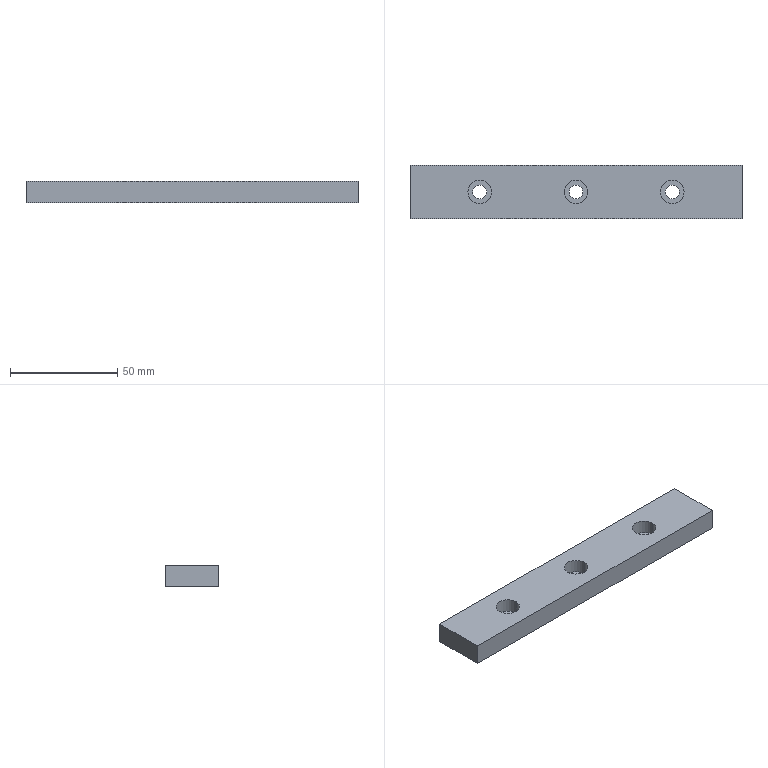Part | STEP file | 0232_213_Plate | 1 solid | 21 faces | box 155 x 25 x 10 mm | volume 36548 mm3 | cylinder 12 | plane 9 | commonest cylinder face diameters 6.5 x6 11 x6
STEP:
#1=CARTESIAN_POINT('',(0.,0.,0.));
#2=DIRECTION('',(0.,0.,1.));
#3=DIRECTION('',(1.,0.,0.));
#4=AXIS2_PLACEMENT_3D('',#1,#2,#3);
#5=CARTESIAN_POINT('',(-39.5,12.5,3.5));
#6=VERTEX_POINT('',#5);
#7=CARTESIAN_POINT('',(-39.5,12.5,10.));
#8=VERTEX_POINT('',#7);
#9=CARTESIAN_POINT('',(-39.5,12.5,10.));
#10=DIRECTION('',(0.,0.,1.));
#11=VECTOR('',#10,1.);
#12=LINE('',#9,#11);
#13=CARTESIAN_POINT('',(-45.,12.5,10.));
#14=DIRECTION('',(0.,0.,1.));
#15=DIRECTION('',(1.,0.,0.));
#16=AXIS2_PLACEMENT_3D('',#13,#14,#15);
#17=CYLINDRICAL_SURFACE('',#16,5.5);
#18=CARTESIAN_POINT('',(6.283,0.));
#19=DIRECTION('',(0.,1.));
#20=VECTOR('',#19,1.);
#21=LINE('',#18,#20);
#22=(GEOMETRIC_REPRESENTATION_CONTEXT(2)PARAMETRIC_REPRESENTATION_CONTEXT()REPRESENTATION_CONTEXT('',''));
#23=DEFINITIONAL_REPRESENTATION('',(#21),#22);
#24=PCURVE('',#17,#23);
#25=CARTESIAN_POINT('',(-45.,12.5,10.));
#26=DIRECTION('',(0.,0.,1.));
#27=DIRECTION('',(1.,0.,0.));
#28=AXIS2_PLACEMENT_3D('',#25,#26,#27);
#29=CYLINDRICAL_SURFACE('',#28,5.5);
#30=CARTESIAN_POINT('',(0.,0.));
#31=DIRECTION('',(0.,1.));
#32=VECTOR('',#31,1.);
#33=LINE('',#30,#32);
#34=(GEOMETRIC_REPRESENTATION_CONTEXT(2)PARAMETRIC_REPRESENTATION_CONTEXT()REPRESENTATION_CONTEXT('',''));
#35=DEFINITIONAL_REPRESENTATION('',(#33),#34);
#36=PCURVE('',#29,#35);
#37=SURFACE_CURVE('',#12,(#24,#36),.PCURVE_S1.);
#38=EDGE_CURVE('',#6,#8,#37,.T.);
#39=ORIENTED_EDGE('',*,*,#38,.T.);
#40=CARTESIAN_POINT('',(-50.5,12.5,10.));
#41=VERTEX_POINT('',#40);
#42=CARTESIAN_POINT('',(-45.,12.5,10.));
#43=DIRECTION('',(0.,0.,1.));
#44=DIRECTION('',(1.,0.,0.));
#45=AXIS2_PLACEMENT_3D('',#42,#43,#44);
#46=CIRCLE('',#45,5.5);
#47=CARTESIAN_POINT('',(0.,0.));
#48=DIRECTION('',(1.,0.));
#49=VECTOR('',#48,1.);
#50=LINE('',#47,#49);
#51=(GEOMETRIC_REPRESENTATION_CONTEXT(2)PARAMETRIC_REPRESENTATION_CONTEXT()REPRESENTATION_CONTEXT('',''));
#52=DEFINITIONAL_REPRESENTATION('',(#50),#51);
#53=PCURVE('',#17,#52);
#54=CARTESIAN_POINT('',(-77.5,0.,10.));
#55=DIRECTION('',(0.,0.,1.));
#56=DIRECTION('',(1.,0.,0.));
#57=AXIS2_PLACEMENT_3D('',#54,#55,#56);
#58=PLANE('',#57);
#59=CARTESIAN_POINT('',(32.5,12.5));
#60=DIRECTION('',(1.,0.));
#61=AXIS2_PLACEMENT_2D('',#59,#60);
#62=CIRCLE('',#61,5.5);
#63=(GEOMETRIC_REPRESENTATION_CONTEXT(2)PARAMETRIC_REPRESENTATION_CONTEXT()REPRESENTATION_CONTEXT('',''));
#64=DEFINITIONAL_REPRESENTATION('',(#62),#63);
#65=PCURVE('',#58,#64);
#66=SURFACE_CURVE('',#46,(#53,#65),.PCURVE_S1.);
#67=EDGE_CURVE('',#41,#8,#66,.T.);
#68=ORIENTED_EDGE('',*,*,#67,.F.);
#69=CARTESIAN_POINT('',(-50.5,12.5,3.5));
#70=VERTEX_POINT('',#69);
#71=CARTESIAN_POINT('',(-50.5,12.5,10.));
#72=DIRECTION('',(0.,0.,1.));
#73=VECTOR('',#72,1.);
#74=LINE('',#71,#73);
#75=CARTESIAN_POINT('',(3.142,0.));
#76=DIRECTION('',(0.,1.));
#77=VECTOR('',#76,1.);
#78=LINE('',#75,#77);
#79=(GEOMETRIC_REPRESENTATION_CONTEXT(2)PARAMETRIC_REPRESENTATION_CONTEXT()REPRESENTATION_CONTEXT('',''));
#80=DEFINITIONAL_REPRESENTATION('',(#78),#79);
#81=PCURVE('',#17,#80);
#82=CARTESIAN_POINT('',(3.142,0.));
#83=DIRECTION('',(0.,1.));
#84=VECTOR('',#83,1.);
#85=LINE('',#82,#84);
#86=(GEOMETRIC_REPRESENTATION_CONTEXT(2)PARAMETRIC_REPRESENTATION_CONTEXT()REPRESENTATION_CONTEXT('',''));
#87=DEFINITIONAL_REPRESENTATION('',(#85),#86);
#88=PCURVE('',#29,#87);
#89=SURFACE_CURVE('',#74,(#81,#88),.PCURVE_S1.);
#90=EDGE_CURVE('',#70,#41,#89,.T.);
#91=ORIENTED_EDGE('',*,*,#90,.F.);
#92=CARTESIAN_POINT('',(-45.,12.5,3.5));
#93=DIRECTION('',(0.,0.,1.));
#94=DIRECTION('',(1.,0.,0.));
#95=AXIS2_PLACEMENT_3D('',#92,#93,#94);
#96=CIRCLE('',#95,5.5);
#97=CARTESIAN_POINT('',(0.,-6.5));
#98=DIRECTION('',(1.,0.));
#99=VECTOR('',#98,1.);
#100=LINE('',#97,#99);
#101=(GEOMETRIC_REPRESENTATION_CONTEXT(2)PARAMETRIC_REPRESENTATION_CONTEXT()REPRESENTATION_CONTEXT('',''));
#102=DEFINITIONAL_REPRESENTATION('',(#100),#101);
#103=PCURVE('',#17,#102);
#104=CARTESIAN_POINT('',(-41.75,12.5,3.5));
#105=DIRECTION('',(0.,0.,-1.));
#106=DIRECTION('',(-1.,0.,0.));
#107=AXIS2_PLACEMENT_3D('',#104,#105,#106);
#108=PLANE('',#107);
#109=CARTESIAN_POINT('',(-2.25,0.));
#110=CARTESIAN_POINT('',(-2.25,9.526));
#111=CARTESIAN_POINT('',(6.,4.763));
#112=CARTESIAN_POINT('',(14.25,0.));
#113=CARTESIAN_POINT('',(6.,-4.763));
#114=CARTESIAN_POINT('',(-2.25,-9.526));
#115=CARTESIAN_POINT('',(-2.25,0.));
#116=(BOUNDED_CURVE()B_SPLINE_CURVE(2,(#109,#110,#111,#112,#113,#114,#115),.UNSPECIFIED.,.T.,.F.)B_SPLINE_CURVE_WITH_KNOTS((1,2,2,2,2,1),(-2.094,0.,2.094,4.189,6.283,8.378),.UNSPECIFIED.)CURVE()GEOMETRIC_REPRESENTATION_ITEM()RATIONAL_B_SPLINE_CURVE((1.,0.5,1.,0.5,1.,0.5,1.))REPRESENTATION_ITEM(''));
#117=(GEOMETRIC_REPRESENTATION_CONTEXT(2)PARAMETRIC_REPRESENTATION_CONTEXT()REPRESENTATION_CONTEXT('',''));
#118=DEFINITIONAL_REPRESENTATION('',(#116),#117);
#119=PCURVE('',#108,#118);
#120=SURFACE_CURVE('',#96,(#103,#119),.PCURVE_S1.);
#121=EDGE_CURVE('',#70,#6,#120,.T.);
#122=ORIENTED_EDGE('',*,*,#121,.T.);
#123=EDGE_LOOP('',(#39,#68,#91,#122));
#124=FACE_BOUND('',#123,.F.);
#125=ADVANCED_FACE('',(#124),#17,.F.);
#126=CARTESIAN_POINT('',(-41.75,12.5,0.));
#127=VERTEX_POINT('',#126);
#128=CARTESIAN_POINT('',(-41.75,12.5,3.5));
#129=VERTEX_POINT('',#128);
#130=CARTESIAN_POINT('',(-41.75,12.5,10.));
#131=DIRECTION('',(0.,0.,1.));
#132=VECTOR('',#131,1.);
#133=LINE('',#130,#132);
#134=CARTESIAN_POINT('',(-45.,12.5,10.));
#135=DIRECTION('',(0.,0.,1.));
#136=DIRECTION('',(1.,0.,0.));
#137=AXIS2_PLACEMENT_3D('',#134,#135,#136);
#138=CYLINDRICAL_SURFACE('',#137,3.25);
#139=CARTESIAN_POINT('',(6.283,0.));
#140=DIRECTION('',(0.,1.));
#141=VECTOR('',#140,1.);
#142=LINE('',#139,#141);
#143=(GEOMETRIC_REPRESENTATION_CONTEXT(2)PARAMETRIC_REPRESENTATION_CONTEXT()REPRESENTATION_CONTEXT('',''));
#144=DEFINITIONAL_REPRESENTATION('',(#142),#143);
#145=PCURVE('',#138,#144);
#146=CARTESIAN_POINT('',(-45.,12.5,10.));
#147=DIRECTION('',(0.,0.,1.));
#148=DIRECTION('',(1.,0.,0.));
#149=AXIS2_PLACEMENT_3D('',#146,#147,#148);
#150=CYLINDRICAL_SURFACE('',#149,3.25);
#151=CARTESIAN_POINT('',(0.,0.));
#152=DIRECTION('',(0.,1.));
#153=VECTOR('',#152,1.);
#154=LINE('',#151,#153);
#155=(GEOMETRIC_REPRESENTATION_CONTEXT(2)PARAMETRIC_REPRESENTATION_CONTEXT()REPRESENTATION_CONTEXT('',''));
#156=DEFINITIONAL_REPRESENTATION('',(#154),#155);
#157=PCURVE('',#150,#156);
#158=SURFACE_CURVE('',#133,(#145,#157),.PCURVE_S1.);
#159=EDGE_CURVE('',#127,#129,#158,.T.);
#160=ORIENTED_EDGE('',*,*,#159,.T.);
#161=CARTESIAN_POINT('',(-48.25,12.5,3.5));
#162=VERTEX_POINT('',#161);
#163=CARTESIAN_POINT('',(-45.,12.5,3.5));
#164=DIRECTION('',(0.,0.,1.));
#165=DIRECTION('',(1.,0.,0.));
#166=AXIS2_PLACEMENT_3D('',#163,#164,#165);
#167=CIRCLE('',#166,3.25);
#168=CARTESIAN_POINT('',(0.,-6.5));
#169=DIRECTION('',(1.,0.));
#170=VECTOR('',#169,1.);
#171=LINE('',#168,#170);
#172=(GEOMETRIC_REPRESENTATION_CONTEXT(2)PARAMETRIC_REPRESENTATION_CONTEXT()REPRESENTATION_CONTEXT('',''));
#173=DEFINITIONAL_REPRESENTATION('',(#171),#172);
#174=PCURVE('',#138,#173);
#175=CARTESIAN_POINT('',(0.,0.));
#176=CARTESIAN_POINT('',(0.,5.629));
#177=CARTESIAN_POINT('',(4.875,2.815));
#178=CARTESIAN_POINT('',(9.75,0.));
#179=CARTESIAN_POINT('',(4.875,-2.815));
#180=CARTESIAN_POINT('',(0.,-5.629));
#181=CARTESIAN_POINT('',(0.,0.));
#182=(BOUNDED_CURVE()B_SPLINE_CURVE(2,(#175,#176,#177,#178,#179,#180,#181),.UNSPECIFIED.,.T.,.F.)B_SPLINE_CURVE_WITH_KNOTS((1,2,2,2,2,1),(-2.094,0.,2.094,4.189,6.283,8.378),.UNSPECIFIED.)CURVE()GEOMETRIC_REPRESENTATION_ITEM()RATIONAL_B_SPLINE_CURVE((1.,0.5,1.,0.5,1.,0.5,1.))REPRESENTATION_ITEM(''));
#183=(GEOMETRIC_REPRESENTATION_CONTEXT(2)PARAMETRIC_REPRESENTATION_CONTEXT()REPRESENTATION_CONTEXT('',''));
#184=DEFINITIONAL_REPRESENTATION('',(#182),#183);
#185=PCURVE('',#108,#184);
#186=SURFACE_CURVE('',#167,(#174,#185),.PCURVE_S1.);
#187=EDGE_CURVE('',#162,#129,#186,.T.);
#188=ORIENTED_EDGE('',*,*,#187,.F.);
#189=CARTESIAN_POINT('',(-48.25,12.5,0.));
#190=VERTEX_POINT('',#189);
#191=CARTESIAN_POINT('',(-48.25,12.5,10.));
#192=DIRECTION('',(0.,0.,1.));
#193=VECTOR('',#192,1.);
#194=LINE('',#191,#193);
#195=CARTESIAN_POINT('',(3.142,0.));
#196=DIRECTION('',(0.,1.));
#197=VECTOR('',#196,1.);
#198=LINE('',#195,#197);
#199=(GEOMETRIC_REPRESENTATION_CONTEXT(2)PARAMETRIC_REPRESENTATION_CONTEXT()REPRESENTATION_CONTEXT('',''));
#200=DEFINITIONAL_REPRESENTATION('',(#198),#199);
#201=PCURVE('',#138,#200);
#202=CARTESIAN_POINT('',(3.142,0.));
#203=DIRECTION('',(0.,1.));
#204=VECTOR('',#203,1.);
#205=LINE('',#202,#204);
#206=(GEOMETRIC_REPRESENTATION_CONTEXT(2)PARAMETRIC_REPRESENTATION_CONTEXT()REPRESENTATION_CONTEXT('',''));
#207=DEFINITIONAL_REPRESENTATION('',(#205),#206);
#208=PCURVE('',#150,#207);
#209=SURFACE_CURVE('',#194,(#201,#208),.PCURVE_S1.);
#210=EDGE_CURVE('',#190,#162,#209,.T.);
#211=ORIENTED_EDGE('',*,*,#210,.F.);
#212=CARTESIAN_POINT('',(-45.,12.5,0.));
#213=DIRECTION('',(0.,0.,1.));
#214=DIRECTION('',(1.,0.,0.));
#215=AXIS2_PLACEMENT_3D('',#212,#213,#214);
#216=CIRCLE('',#215,3.25);
#217=CARTESIAN_POINT('',(0.,-10.));
#218=DIRECTION('',(1.,0.));
#219=VECTOR('',#218,1.);
#220=LINE('',#217,#219);
#221=(GEOMETRIC_REPRESENTATION_CONTEXT(2)PARAMETRIC_REPRESENTATION_CONTEXT()REPRESENTATION_CONTEXT('',''));
#222=DEFINITIONAL_REPRESENTATION('',(#220),#221);
#223=PCURVE('',#138,#222);
#224=CARTESIAN_POINT('',(-77.5,0.,0.));
#225=DIRECTION('',(0.,0.,1.));
#226=DIRECTION('',(1.,0.,0.));
#227=AXIS2_PLACEMENT_3D('',#224,#225,#226);
#228=PLANE('',#227);
#229=CARTESIAN_POINT('',(32.5,12.5));
#230=DIRECTION('',(1.,0.));
#231=AXIS2_PLACEMENT_2D('',#229,#230);
#232=CIRCLE('',#231,3.25);
#233=(GEOMETRIC_REPRESENTATION_CONTEXT(2)PARAMETRIC_REPRESENTATION_CONTEXT()REPRESENTATION_CONTEXT('',''));
#234=DEFINITIONAL_REPRESENTATION('',(#232),#233);
#235=PCURVE('',#228,#234);
#236=SURFACE_CURVE('',#216,(#223,#235),.PCURVE_S1.);
#237=EDGE_CURVE('',#190,#127,#236,.T.);
#238=ORIENTED_EDGE('',*,*,#237,.T.);
#239=EDGE_LOOP('',(#160,#188,#211,#238));
#240=FACE_BOUND('',#239,.F.);
#241=ADVANCED_FACE('',(#240),#138,.F.);
#242=CARTESIAN_POINT('',(5.5,12.5,3.5));
#243=VERTEX_POINT('',#242);
#244=CARTESIAN_POINT('',(5.5,12.5,10.));
#245=VERTEX_POINT('',#244);
#246=CARTESIAN_POINT('',(5.5,12.5,10.));
#247=DIRECTION('',(0.,0.,1.));
#248=VECTOR('',#247,1.);
#249=LINE('',#246,#248);
#250=CARTESIAN_POINT('',(0.,12.5,10.));
#251=DIRECTION('',(0.,0.,1.));
#252=DIRECTION('',(1.,0.,0.));
#253=AXIS2_PLACEMENT_3D('',#250,#251,#252);
#254=CYLINDRICAL_SURFACE('',#253,5.5);
#255=CARTESIAN_POINT('',(6.283,0.));
#256=DIRECTION('',(0.,1.));
#257=VECTOR('',#256,1.);
#258=LINE('',#255,#257);
#259=(GEOMETRIC_REPRESENTATION_CONTEXT(2)PARAMETRIC_REPRESENTATION_CONTEXT()REPRESENTATION_CONTEXT('',''));
#260=DEFINITIONAL_REPRESENTATION('',(#258),#259);
#261=PCURVE('',#254,#260);
#262=CARTESIAN_POINT('',(0.,12.5,10.));
#263=DIRECTION('',(0.,0.,1.));
#264=DIRECTION('',(1.,0.,0.));
#265=AXIS2_PLACEMENT_3D('',#262,#263,#264);
#266=CYLINDRICAL_SURFACE('',#265,5.5);
#267=CARTESIAN_POINT('',(0.,0.));
#268=DIRECTION('',(0.,1.));
#269=VECTOR('',#268,1.);
#270=LINE('',#267,#269);
#271=(GEOMETRIC_REPRESENTATION_CONTEXT(2)PARAMETRIC_REPRESENTATION_CONTEXT()REPRESENTATION_CONTEXT('',''));
#272=DEFINITIONAL_REPRESENTATION('',(#270),#271);
#273=PCURVE('',#266,#272);
#274=SURFACE_CURVE('',#249,(#261,#273),.PCURVE_S1.);
#275=EDGE_CURVE('',#243,#245,#274,.T.);
#276=ORIENTED_EDGE('',*,*,#275,.T.);
#277=CARTESIAN_POINT('',(-5.5,12.5,10.));
#278=VERTEX_POINT('',#277);
#279=CARTESIAN_POINT('',(0.,12.5,10.));
#280=DIRECTION('',(0.,0.,1.));
#281=DIRECTION('',(1.,0.,0.));
#282=AXIS2_PLACEMENT_3D('',#279,#280,#281);
#283=CIRCLE('',#282,5.5);
#284=CARTESIAN_POINT('',(0.,0.));
#285=DIRECTION('',(1.,0.));
#286=VECTOR('',#285,1.);
#287=LINE('',#284,#286);
#288=(GEOMETRIC_REPRESENTATION_CONTEXT(2)PARAMETRIC_REPRESENTATION_CONTEXT()REPRESENTATION_CONTEXT('',''));
#289=DEFINITIONAL_REPRESENTATION('',(#287),#288);
#290=PCURVE('',#254,#289);
#291=CARTESIAN_POINT('',(77.5,12.5));
#292=DIRECTION('',(1.,0.));
#293=AXIS2_PLACEMENT_2D('',#291,#292);
#294=CIRCLE('',#293,5.5);
#295=(GEOMETRIC_REPRESENTATION_CONTEXT(2)PARAMETRIC_REPRESENTATION_CONTEXT()REPRESENTATION_CONTEXT('',''));
#296=DEFINITIONAL_REPRESENTATION('',(#294),#295);
#297=PCURVE('',#58,#296);
#298=SURFACE_CURVE('',#283,(#290,#297),.PCURVE_S1.);
#299=EDGE_CURVE('',#278,#245,#298,.T.);
#300=ORIENTED_EDGE('',*,*,#299,.F.);
#301=CARTESIAN_POINT('',(-5.5,12.5,3.5));
#302=VERTEX_POINT('',#301);
#303=CARTESIAN_POINT('',(-5.5,12.5,10.));
#304=DIRECTION('',(0.,0.,1.));
#305=VECTOR('',#304,1.);
#306=LINE('',#303,#305);
#307=CARTESIAN_POINT('',(3.142,0.));
#308=DIRECTION('',(0.,1.));
#309=VECTOR('',#308,1.);
#310=LINE('',#307,#309);
#311=(GEOMETRIC_REPRESENTATION_CONTEXT(2)PARAMETRIC_REPRESENTATION_CONTEXT()REPRESENTATION_CONTEXT('',''));
#312=DEFINITIONAL_REPRESENTATION('',(#310),#311);
#313=PCURVE('',#254,#312);
#314=CARTESIAN_POINT('',(3.142,0.));
#315=DIRECTION('',(0.,1.));
#316=VECTOR('',#315,1.);
#317=LINE('',#314,#316);
#318=(GEOMETRIC_REPRESENTATION_CONTEXT(2)PARAMETRIC_REPRESENTATION_CONTEXT()REPRESENTATION_CONTEXT('',''));
#319=DEFINITIONAL_REPRESENTATION('',(#317),#318);
#320=PCURVE('',#266,#319);
#321=SURFACE_CURVE('',#306,(#313,#320),.PCURVE_S1.);
#322=EDGE_CURVE('',#302,#278,#321,.T.);
#323=ORIENTED_EDGE('',*,*,#322,.F.);
#324=CARTESIAN_POINT('',(0.,12.5,3.5));
#325=DIRECTION('',(0.,0.,1.));
#326=DIRECTION('',(1.,0.,0.));
#327=AXIS2_PLACEMENT_3D('',#324,#325,#326);
#328=CIRCLE('',#327,5.5);
#329=CARTESIAN_POINT('',(0.,-6.5));
#330=DIRECTION('',(1.,0.));
#331=VECTOR('',#330,1.);
#332=LINE('',#329,#331);
#333=(GEOMETRIC_REPRESENTATION_CONTEXT(2)PARAMETRIC_REPRESENTATION_CONTEXT()REPRESENTATION_CONTEXT('',''));
#334=DEFINITIONAL_REPRESENTATION('',(#332),#333);
#335=PCURVE('',#254,#334);
#336=CARTESIAN_POINT('',(3.25,12.5,3.5));
#337=DIRECTION('',(0.,0.,-1.));
#338=DIRECTION('',(-1.,0.,0.));
#339=AXIS2_PLACEMENT_3D('',#336,#337,#338);
#340=PLANE('',#339);
#341=CARTESIAN_POINT('',(-2.25,0.));
#342=CARTESIAN_POINT('',(-2.25,9.526));
#343=CARTESIAN_POINT('',(6.,4.763));
#344=CARTESIAN_POINT('',(14.25,0.));
#345=CARTESIAN_POINT('',(6.,-4.763));
#346=CARTESIAN_POINT('',(-2.25,-9.526));
#347=CARTESIAN_POINT('',(-2.25,0.));
#348=(BOUNDED_CURVE()B_SPLINE_CURVE(2,(#341,#342,#343,#344,#345,#346,#347),.UNSPECIFIED.,.T.,.F.)B_SPLINE_CURVE_WITH_KNOTS((1,2,2,2,2,1),(-2.094,0.,2.094,4.189,6.283,8.378),.UNSPECIFIED.)CURVE()GEOMETRIC_REPRESENTATION_ITEM()RATIONAL_B_SPLINE_CURVE((1.,0.5,1.,0.5,1.,0.5,1.))REPRESENTATION_ITEM(''));
#349=(GEOMETRIC_REPRESENTATION_CONTEXT(2)PARAMETRIC_REPRESENTATION_CONTEXT()REPRESENTATION_CONTEXT('',''));
#350=DEFINITIONAL_REPRESENTATION('',(#348),#349);
#351=PCURVE('',#340,#350);
#352=SURFACE_CURVE('',#328,(#335,#351),.PCURVE_S1.);
#353=EDGE_CURVE('',#302,#243,#352,.T.);
#354=ORIENTED_EDGE('',*,*,#353,.T.);
#355=EDGE_LOOP('',(#276,#300,#323,#354));
#356=FACE_BOUND('',#355,.F.);
#357=ADVANCED_FACE('',(#356),#254,.F.);
#358=CARTESIAN_POINT('',(3.25,12.5,0.));
#359=VERTEX_POINT('',#358);
#360=CARTESIAN_POINT('',(3.25,12.5,3.5));
#361=VERTEX_POINT('',#360);
#362=CARTESIAN_POINT('',(3.25,12.5,10.));
#363=DIRECTION('',(0.,0.,1.));
#364=VECTOR('',#363,1.);
#365=LINE('',#362,#364);
#366=CARTESIAN_POINT('',(0.,12.5,10.));
#367=DIRECTION('',(0.,0.,1.));
#368=DIRECTION('',(1.,0.,0.));
#369=AXIS2_PLACEMENT_3D('',#366,#367,#368);
#370=CYLINDRICAL_SURFACE('',#369,3.25);
#371=CARTESIAN_POINT('',(6.283,0.));
#372=DIRECTION('',(0.,1.));
#373=VECTOR('',#372,1.);
#374=LINE('',#371,#373);
#375=(GEOMETRIC_REPRESENTATION_CONTEXT(2)PARAMETRIC_REPRESENTATION_CONTEXT()REPRESENTATION_CONTEXT('',''));
#376=DEFINITIONAL_REPRESENTATION('',(#374),#375);
#377=PCURVE('',#370,#376);
#378=CARTESIAN_POINT('',(0.,12.5,10.));
#379=DIRECTION('',(0.,0.,1.));
#380=DIRECTION('',(1.,0.,0.));
#381=AXIS2_PLACEMENT_3D('',#378,#379,#380);
#382=CYLINDRICAL_SURFACE('',#381,3.25);
#383=CARTESIAN_POINT('',(0.,0.));
#384=DIRECTION('',(0.,1.));
#385=VECTOR('',#384,1.);
#386=LINE('',#383,#385);
#387=(GEOMETRIC_REPRESENTATION_CONTEXT(2)PARAMETRIC_REPRESENTATION_CONTEXT()REPRESENTATION_CONTEXT('',''));
#388=DEFINITIONAL_REPRESENTATION('',(#386),#387);
#389=PCURVE('',#382,#388);
#390=SURFACE_CURVE('',#365,(#377,#389),.PCURVE_S1.);
#391=EDGE_CURVE('',#359,#361,#390,.T.);
#392=ORIENTED_EDGE('',*,*,#391,.T.);
#393=CARTESIAN_POINT('',(-3.25,12.5,3.5));
#394=VERTEX_POINT('',#393);
#395=CARTESIAN_POINT('',(0.,12.5,3.5));
#396=DIRECTION('',(0.,0.,1.));
#397=DIRECTION('',(1.,0.,0.));
#398=AXIS2_PLACEMENT_3D('',#395,#396,#397);
#399=CIRCLE('',#398,3.25);
#400=CARTESIAN_POINT('',(0.,-6.5));
#401=DIRECTION('',(1.,0.));
#402=VECTOR('',#401,1.);
#403=LINE('',#400,#402);
#404=(GEOMETRIC_REPRESENTATION_CONTEXT(2)PARAMETRIC_REPRESENTATION_CONTEXT()REPRESENTATION_CONTEXT('',''));
#405=DEFINITIONAL_REPRESENTATION('',(#403),#404);
#406=PCURVE('',#370,#405);
#407=CARTESIAN_POINT('',(0.,0.));
#408=CARTESIAN_POINT('',(0.,5.629));
#409=CARTESIAN_POINT('',(4.875,2.815));
#410=CARTESIAN_POINT('',(9.75,0.));
#411=CARTESIAN_POINT('',(4.875,-2.815));
#412=CARTESIAN_POINT('',(0.,-5.629));
#413=CARTESIAN_POINT('',(0.,0.));
#414=(BOUNDED_CURVE()B_SPLINE_CURVE(2,(#407,#408,#409,#410,#411,#412,#413),.UNSPECIFIED.,.T.,.F.)B_SPLINE_CURVE_WITH_KNOTS((1,2,2,2,2,1),(-2.094,0.,2.094,4.189,6.283,8.378),.UNSPECIFIED.)CURVE()GEOMETRIC_REPRESENTATION_ITEM()RATIONAL_B_SPLINE_CURVE((1.,0.5,1.,0.5,1.,0.5,1.))REPRESENTATION_ITEM(''));
#415=(GEOMETRIC_REPRESENTATION_CONTEXT(2)PARAMETRIC_REPRESENTATION_CONTEXT()REPRESENTATION_CONTEXT('',''));
#416=DEFINITIONAL_REPRESENTATION('',(#414),#415);
#417=PCURVE('',#340,#416);
#418=SURFACE_CURVE('',#399,(#406,#417),.PCURVE_S1.);
#419=EDGE_CURVE('',#394,#361,#418,.T.);
#420=ORIENTED_EDGE('',*,*,#419,.F.);
#421=CARTESIAN_POINT('',(-3.25,12.5,0.));
#422=VERTEX_POINT('',#421);
#423=CARTESIAN_POINT('',(-3.25,12.5,10.));
#424=DIRECTION('',(0.,0.,1.));
#425=VECTOR('',#424,1.);
#426=LINE('',#423,#425);
#427=CARTESIAN_POINT('',(3.142,0.));
#428=DIRECTION('',(0.,1.));
#429=VECTOR('',#428,1.);
#430=LINE('',#427,#429);
#431=(GEOMETRIC_REPRESENTATION_CONTEXT(2)PARAMETRIC_REPRESENTATION_CONTEXT()REPRESENTATION_CONTEXT('',''));
#432=DEFINITIONAL_REPRESENTATION('',(#430),#431);
#433=PCURVE('',#370,#432);
#434=CARTESIAN_POINT('',(3.142,0.));
#435=DIRECTION('',(0.,1.));
#436=VECTOR('',#435,1.);
#437=LINE('',#434,#436);
#438=(GEOMETRIC_REPRESENTATION_CONTEXT(2)PARAMETRIC_REPRESENTATION_CONTEXT()REPRESENTATION_CONTEXT('',''));
#439=DEFINITIONAL_REPRESENTATION('',(#437),#438);
#440=PCURVE('',#382,#439);
#441=SURFACE_CURVE('',#426,(#433,#440),.PCURVE_S1.);
#442=EDGE_CURVE('',#422,#394,#441,.T.);
#443=ORIENTED_EDGE('',*,*,#442,.F.);
#444=CARTESIAN_POINT('',(0.,12.5,0.));
#445=DIRECTION('',(0.,0.,1.));
#446=DIRECTION('',(1.,0.,0.));
#447=AXIS2_PLACEMENT_3D('',#444,#445,#446);
#448=CIRCLE('',#447,3.25);
#449=CARTESIAN_POINT('',(0.,-10.));
#450=DIRECTION('',(1.,0.));
#451=VECTOR('',#450,1.);
#452=LINE('',#449,#451);
#453=(GEOMETRIC_REPRESENTATION_CONTEXT(2)PARAMETRIC_REPRESENTATION_CONTEXT()REPRESENTATION_CONTEXT('',''));
#454=DEFINITIONAL_REPRESENTATION('',(#452),#453);
#455=PCURVE('',#370,#454);
#456=CARTESIAN_POINT('',(77.5,12.5));
#457=DIRECTION('',(1.,0.));
#458=AXIS2_PLACEMENT_2D('',#456,#457);
#459=CIRCLE('',#458,3.25);
#460=(GEOMETRIC_REPRESENTATION_CONTEXT(2)PARAMETRIC_REPRESENTATION_CONTEXT()REPRESENTATION_CONTEXT('',''));
#461=DEFINITIONAL_REPRESENTATION('',(#459),#460);
#462=PCURVE('',#228,#461);
#463=SURFACE_CURVE('',#448,(#455,#462),.PCURVE_S1.);
#464=EDGE_CURVE('',#422,#359,#463,.T.);
#465=ORIENTED_EDGE('',*,*,#464,.T.);
#466=EDGE_LOOP('',(#392,#420,#443,#465));
#467=FACE_BOUND('',#466,.F.);
#468=ADVANCED_FACE('',(#467),#370,.F.);
#469=CARTESIAN_POINT('',(50.5,12.5,3.5));
#470=VERTEX_POINT('',#469);
#471=CARTESIAN_POINT('',(50.5,12.5,10.));
#472=VERTEX_POINT('',#471);
#473=CARTESIAN_POINT('',(50.5,12.5,10.));
#474=DIRECTION('',(0.,0.,1.));
#475=VECTOR('',#474,1.);
#476=LINE('',#473,#475);
#477=CARTESIAN_POINT('',(45.,12.5,10.));
#478=DIRECTION('',(0.,0.,1.));
#479=DIRECTION('',(1.,0.,0.));
#480=AXIS2_PLACEMENT_3D('',#477,#478,#479);
#481=CYLINDRICAL_SURFACE('',#480,5.5);
#482=CARTESIAN_POINT('',(6.283,0.));
#483=DIRECTION('',(0.,1.));
#484=VECTOR('',#483,1.);
#485=LINE('',#482,#484);
#486=(GEOMETRIC_REPRESENTATION_CONTEXT(2)PARAMETRIC_REPRESENTATION_CONTEXT()REPRESENTATION_CONTEXT('',''));
#487=DEFINITIONAL_REPRESENTATION('',(#485),#486);
#488=PCURVE('',#481,#487);
#489=CARTESIAN_POINT('',(45.,12.5,10.));
#490=DIRECTION('',(0.,0.,1.));
#491=DIRECTION('',(1.,0.,0.));
#492=AXIS2_PLACEMENT_3D('',#489,#490,#491);
#493=CYLINDRICAL_SURFACE('',#492,5.5);
#494=CARTESIAN_POINT('',(0.,0.));
#495=DIRECTION('',(0.,1.));
#496=VECTOR('',#495,1.);
#497=LINE('',#494,#496);
#498=(GEOMETRIC_REPRESENTATION_CONTEXT(2)PARAMETRIC_REPRESENTATION_CONTEXT()REPRESENTATION_CONTEXT('',''));
#499=DEFINITIONAL_REPRESENTATION('',(#497),#498);
#500=PCURVE('',#493,#499);
#501=SURFACE_CURVE('',#476,(#488,#500),.PCURVE_S1.);
#502=EDGE_CURVE('',#470,#472,#501,.T.);
#503=ORIENTED_EDGE('',*,*,#502,.T.);
#504=CARTESIAN_POINT('',(39.5,12.5,10.));
#505=VERTEX_POINT('',#504);
#506=CARTESIAN_POINT('',(45.,12.5,10.));
#507=DIRECTION('',(0.,0.,1.));
#508=DIRECTION('',(1.,0.,0.));
#509=AXIS2_PLACEMENT_3D('',#506,#507,#508);
#510=CIRCLE('',#509,5.5);
#511=CARTESIAN_POINT('',(0.,0.));
#512=DIRECTION('',(1.,0.));
#513=VECTOR('',#512,1.);
#514=LINE('',#511,#513);
#515=(GEOMETRIC_REPRESENTATION_CONTEXT(2)PARAMETRIC_REPRESENTATION_CONTEXT()REPRESENTATION_CONTEXT('',''));
#516=DEFINITIONAL_REPRESENTATION('',(#514),#515);
#517=PCURVE('',#481,#516);
#518=CARTESIAN_POINT('',(122.5,12.5));
#519=DIRECTION('',(1.,0.));
#520=AXIS2_PLACEMENT_2D('',#518,#519);
#521=CIRCLE('',#520,5.5);
#522=(GEOMETRIC_REPRESENTATION_CONTEXT(2)PARAMETRIC_REPRESENTATION_CONTEXT()REPRESENTATION_CONTEXT('',''));
#523=DEFINITIONAL_REPRESENTATION('',(#521),#522);
#524=PCURVE('',#58,#523);
#525=SURFACE_CURVE('',#510,(#517,#524),.PCURVE_S1.);
#526=EDGE_CURVE('',#505,#472,#525,.T.);
#527=ORIENTED_EDGE('',*,*,#526,.F.);
#528=CARTESIAN_POINT('',(39.5,12.5,3.5));
#529=VERTEX_POINT('',#528);
#530=CARTESIAN_POINT('',(39.5,12.5,10.));
#531=DIRECTION('',(0.,0.,1.));
#532=VECTOR('',#531,1.);
#533=LINE('',#530,#532);
#534=CARTESIAN_POINT('',(3.142,0.));
#535=DIRECTION('',(0.,1.));
#536=VECTOR('',#535,1.);
#537=LINE('',#534,#536);
#538=(GEOMETRIC_REPRESENTATION_CONTEXT(2)PARAMETRIC_REPRESENTATION_CONTEXT()REPRESENTATION_CONTEXT('',''));
#539=DEFINITIONAL_REPRESENTATION('',(#537),#538);
#540=PCURVE('',#481,#539);
#541=CARTESIAN_POINT('',(3.142,0.));
#542=DIRECTION('',(0.,1.));
#543=VECTOR('',#542,1.);
#544=LINE('',#541,#543);
#545=(GEOMETRIC_REPRESENTATION_CONTEXT(2)PARAMETRIC_REPRESENTATION_CONTEXT()REPRESENTATION_CONTEXT('',''));
#546=DEFINITIONAL_REPRESENTATION('',(#544),#545);
#547=PCURVE('',#493,#546);
#548=SURFACE_CURVE('',#533,(#540,#547),.PCURVE_S1.);
#549=EDGE_CURVE('',#529,#505,#548,.T.);
#550=ORIENTED_EDGE('',*,*,#549,.F.);
#551=CARTESIAN_POINT('',(45.,12.5,3.5));
#552=DIRECTION('',(0.,0.,1.));
#553=DIRECTION('',(1.,0.,0.));
#554=AXIS2_PLACEMENT_3D('',#551,#552,#553);
#555=CIRCLE('',#554,5.5);
#556=CARTESIAN_POINT('',(0.,-6.5));
#557=DIRECTION('',(1.,0.));
#558=VECTOR('',#557,1.);
#559=LINE('',#556,#558);
#560=(GEOMETRIC_REPRESENTATION_CONTEXT(2)PARAMETRIC_REPRESENTATION_CONTEXT()REPRESENTATION_CONTEXT('',''));
#561=DEFINITIONAL_REPRESENTATION('',(#559),#560);
#562=PCURVE('',#481,#561);
#563=CARTESIAN_POINT('',(48.25,12.5,3.5));
#564=DIRECTION('',(0.,0.,-1.));
#565=DIRECTION('',(-1.,0.,0.));
#566=AXIS2_PLACEMENT_3D('',#563,#564,#565);
#567=PLANE('',#566);
#568=CARTESIAN_POINT('',(-2.25,0.));
#569=CARTESIAN_POINT('',(-2.25,9.526));
#570=CARTESIAN_POINT('',(6.,4.763));
#571=CARTESIAN_POINT('',(14.25,0.));
#572=CARTESIAN_POINT('',(6.,-4.763));
#573=CARTESIAN_POINT('',(-2.25,-9.526));
#574=CARTESIAN_POINT('',(-2.25,0.));
#575=(BOUNDED_CURVE()B_SPLINE_CURVE(2,(#568,#569,#570,#571,#572,#573,#574),.UNSPECIFIED.,.T.,.F.)B_SPLINE_CURVE_WITH_KNOTS((1,2,2,2,2,1),(-2.094,0.,2.094,4.189,6.283,8.378),.UNSPECIFIED.)CURVE()GEOMETRIC_REPRESENTATION_ITEM()RATIONAL_B_SPLINE_CURVE((1.,0.5,1.,0.5,1.,0.5,1.))REPRESENTATION_ITEM(''));
#576=(GEOMETRIC_REPRESENTATION_CONTEXT(2)PARAMETRIC_REPRESENTATION_CONTEXT()REPRESENTATION_CONTEXT('',''));
#577=DEFINITIONAL_REPRESENTATION('',(#575),#576);
#578=PCURVE('',#567,#577);
#579=SURFACE_CURVE('',#555,(#562,#578),.PCURVE_S1.);
#580=EDGE_CURVE('',#529,#470,#579,.T.);
#581=ORIENTED_EDGE('',*,*,#580,.T.);
#582=EDGE_LOOP('',(#503,#527,#550,#581));
#583=FACE_BOUND('',#582,.F.);
#584=ADVANCED_FACE('',(#583),#481,.F.);
#585=CARTESIAN_POINT('',(48.25,12.5,0.));
#586=VERTEX_POINT('',#585);
#587=CARTESIAN_POINT('',(48.25,12.5,3.5));
#588=VERTEX_POINT('',#587);
#589=CARTESIAN_POINT('',(48.25,12.5,10.));
#590=DIRECTION('',(0.,0.,1.));
#591=VECTOR('',#590,1.);
#592=LINE('',#589,#591);
#593=CARTESIAN_POINT('',(45.,12.5,10.));
#594=DIRECTION('',(0.,0.,1.));
#595=DIRECTION('',(1.,0.,0.));
#596=AXIS2_PLACEMENT_3D('',#593,#594,#595);
#597=CYLINDRICAL_SURFACE('',#596,3.25);
#598=CARTESIAN_POINT('',(6.283,0.));
#599=DIRECTION('',(0.,1.));
#600=VECTOR('',#599,1.);
#601=LINE('',#598,#600);
#602=(GEOMETRIC_REPRESENTATION_CONTEXT(2)PARAMETRIC_REPRESENTATION_CONTEXT()REPRESENTATION_CONTEXT('',''));
#603=DEFINITIONAL_REPRESENTATION('',(#601),#602);
#604=PCURVE('',#597,#603);
#605=CARTESIAN_POINT('',(45.,12.5,10.));
#606=DIRECTION('',(0.,0.,1.));
#607=DIRECTION('',(1.,0.,0.));
#608=AXIS2_PLACEMENT_3D('',#605,#606,#607);
#609=CYLINDRICAL_SURFACE('',#608,3.25);
#610=CARTESIAN_POINT('',(0.,0.));
#611=DIRECTION('',(0.,1.));
#612=VECTOR('',#611,1.);
#613=LINE('',#610,#612);
#614=(GEOMETRIC_REPRESENTATION_CONTEXT(2)PARAMETRIC_REPRESENTATION_CONTEXT()REPRESENTATION_CONTEXT('',''));
#615=DEFINITIONAL_REPRESENTATION('',(#613),#614);
#616=PCURVE('',#609,#615);
#617=SURFACE_CURVE('',#592,(#604,#616),.PCURVE_S1.);
#618=EDGE_CURVE('',#586,#588,#617,.T.);
#619=ORIENTED_EDGE('',*,*,#618,.T.);
#620=CARTESIAN_POINT('',(41.75,12.5,3.5));
#621=VERTEX_POINT('',#620);
#622=CARTESIAN_POINT('',(45.,12.5,3.5));
#623=DIRECTION('',(0.,0.,1.));
#624=DIRECTION('',(1.,0.,0.));
#625=AXIS2_PLACEMENT_3D('',#622,#623,#624);
#626=CIRCLE('',#625,3.25);
#627=CARTESIAN_POINT('',(0.,-6.5));
#628=DIRECTION('',(1.,0.));
#629=VECTOR('',#628,1.);
#630=LINE('',#627,#629);
#631=(GEOMETRIC_REPRESENTATION_CONTEXT(2)PARAMETRIC_REPRESENTATION_CONTEXT()REPRESENTATION_CONTEXT('',''));
#632=DEFINITIONAL_REPRESENTATION('',(#630),#631);
#633=PCURVE('',#597,#632);
#634=CARTESIAN_POINT('',(0.,0.));
#635=CARTESIAN_POINT('',(0.,5.629));
#636=CARTESIAN_POINT('',(4.875,2.815));
#637=CARTESIAN_POINT('',(9.75,0.));
#638=CARTESIAN_POINT('',(4.875,-2.815));
#639=CARTESIAN_POINT('',(0.,-5.629));
#640=CARTESIAN_POINT('',(0.,0.));
#641=(BOUNDED_CURVE()B_SPLINE_CURVE(2,(#634,#635,#636,#637,#638,#639,#640),.UNSPECIFIED.,.T.,.F.)B_SPLINE_CURVE_WITH_KNOTS((1,2,2,2,2,1),(-2.094,0.,2.094,4.189,6.283,8.378),.UNSPECIFIED.)CURVE()GEOMETRIC_REPRESENTATION_ITEM()RATIONAL_B_SPLINE_CURVE((1.,0.5,1.,0.5,1.,0.5,1.))REPRESENTATION_ITEM(''));
#642=(GEOMETRIC_REPRESENTATION_CONTEXT(2)PARAMETRIC_REPRESENTATION_CONTEXT()REPRESENTATION_CONTEXT('',''));
#643=DEFINITIONAL_REPRESENTATION('',(#641),#642);
#644=PCURVE('',#567,#643);
#645=SURFACE_CURVE('',#626,(#633,#644),.PCURVE_S1.);
#646=EDGE_CURVE('',#621,#588,#645,.T.);
#647=ORIENTED_EDGE('',*,*,#646,.F.);
#648=CARTESIAN_POINT('',(41.75,12.5,0.));
#649=VERTEX_POINT('',#648);
#650=CARTESIAN_POINT('',(41.75,12.5,10.));
#651=DIRECTION('',(0.,0.,1.));
#652=VECTOR('',#651,1.);
#653=LINE('',#650,#652);
#654=CARTESIAN_POINT('',(3.142,0.));
#655=DIRECTION('',(0.,1.));
#656=VECTOR('',#655,1.);
#657=LINE('',#654,#656);
#658=(GEOMETRIC_REPRESENTATION_CONTEXT(2)PARAMETRIC_REPRESENTATION_CONTEXT()REPRESENTATION_CONTEXT('',''));
#659=DEFINITIONAL_REPRESENTATION('',(#657),#658);
#660=PCURVE('',#597,#659);
#661=CARTESIAN_POINT('',(3.142,0.));
#662=DIRECTION('',(0.,1.));
#663=VECTOR('',#662,1.);
#664=LINE('',#661,#663);
#665=(GEOMETRIC_REPRESENTATION_CONTEXT(2)PARAMETRIC_REPRESENTATION_CONTEXT()REPRESENTATION_CONTEXT('',''));
#666=DEFINITIONAL_REPRESENTATION('',(#664),#665);
#667=PCURVE('',#609,#666);
#668=SURFACE_CURVE('',#653,(#660,#667),.PCURVE_S1.);
#669=EDGE_CURVE('',#649,#621,#668,.T.);
#670=ORIENTED_EDGE('',*,*,#669,.F.);
#671=CARTESIAN_POINT('',(45.,12.5,0.));
#672=DIRECTION('',(0.,0.,1.));
#673=DIRECTION('',(1.,0.,0.));
#674=AXIS2_PLACEMENT_3D('',#671,#672,#673);
#675=CIRCLE('',#674,3.25);
#676=CARTESIAN_POINT('',(0.,-10.));
#677=DIRECTION('',(1.,0.));
#678=VECTOR('',#677,1.);
#679=LINE('',#676,#678);
#680=(GEOMETRIC_REPRESENTATION_CONTEXT(2)PARAMETRIC_REPRESENTATION_CONTEXT()REPRESENTATION_CONTEXT('',''));
#681=DEFINITIONAL_REPRESENTATION('',(#679),#680);
#682=PCURVE('',#597,#681);
#683=CARTESIAN_POINT('',(122.5,12.5));
#684=DIRECTION('',(1.,0.));
#685=AXIS2_PLACEMENT_2D('',#683,#684);
#686=CIRCLE('',#685,3.25);
#687=(GEOMETRIC_REPRESENTATION_CONTEXT(2)PARAMETRIC_REPRESENTATION_CONTEXT()REPRESENTATION_CONTEXT('',''));
#688=DEFINITIONAL_REPRESENTATION('',(#686),#687);
#689=PCURVE('',#228,#688);
#690=SURFACE_CURVE('',#675,(#682,#689),.PCURVE_S1.);
#691=EDGE_CURVE('',#649,#586,#690,.T.);
#692=ORIENTED_EDGE('',*,*,#691,.T.);
#693=EDGE_LOOP('',(#619,#647,#670,#692));
#694=FACE_BOUND('',#693,.F.);
#695=ADVANCED_FACE('',(#694),#597,.F.);
#696=CARTESIAN_POINT('',(-77.5,25.,0.));
#697=VERTEX_POINT('',#696);
#698=CARTESIAN_POINT('',(-77.5,0.,0.));
#699=VERTEX_POINT('',#698);
#700=CARTESIAN_POINT('',(-77.5,25.,0.));
#701=DIRECTION('',(0.,-1.,0.));
#702=VECTOR('',#701,1.);
#703=LINE('',#700,#702);
#704=CARTESIAN_POINT('',(-77.5,25.,10.));
#705=DIRECTION('',(1.,0.,0.));
#706=DIRECTION('',(0.,1.,0.));
#707=AXIS2_PLACEMENT_3D('',#704,#705,#706);
#708=PLANE('',#707);
#709=CARTESIAN_POINT('',(0.,-10.));
#710=DIRECTION('',(-1.,0.));
#711=VECTOR('',#710,1.);
#712=LINE('',#709,#711);
#713=(GEOMETRIC_REPRESENTATION_CONTEXT(2)PARAMETRIC_REPRESENTATION_CONTEXT()REPRESENTATION_CONTEXT('',''));
#714=DEFINITIONAL_REPRESENTATION('',(#712),#713);
#715=PCURVE('',#708,#714);
#716=CARTESIAN_POINT('',(0.,25.));
#717=DIRECTION('',(0.,-1.));
#718=VECTOR('',#717,1.);
#719=LINE('',#716,#718);
#720=(GEOMETRIC_REPRESENTATION_CONTEXT(2)PARAMETRIC_REPRESENTATION_CONTEXT()REPRESENTATION_CONTEXT('',''));
#721=DEFINITIONAL_REPRESENTATION('',(#719),#720);
#722=PCURVE('',#228,#721);
#723=SURFACE_CURVE('',#703,(#715,#722),.PCURVE_S1.);
#724=EDGE_CURVE('',#697,#699,#723,.T.);
#725=ORIENTED_EDGE('',*,*,#724,.T.);
#726=CARTESIAN_POINT('',(-77.5,0.,10.));
#727=VERTEX_POINT('',#726);
#728=CARTESIAN_POINT('',(-77.5,0.,10.));
#729=DIRECTION('',(0.,0.,-1.));
#730=VECTOR('',#729,1.);
#731=LINE('',#728,#730);
#732=CARTESIAN_POINT('',(-25.,0.));
#733=DIRECTION('',(0.,-1.));
#734=VECTOR('',#733,1.);
#735=LINE('',#732,#734);
#736=(GEOMETRIC_REPRESENTATION_CONTEXT(2)PARAMETRIC_REPRESENTATION_CONTEXT()REPRESENTATION_CONTEXT('',''));
#737=DEFINITIONAL_REPRESENTATION('',(#735),#736);
#738=PCURVE('',#708,#737);
#739=CARTESIAN_POINT('',(-77.5,0.,10.));
#740=DIRECTION('',(0.,1.,0.));
#741=DIRECTION('',(0.,0.,1.));
#742=AXIS2_PLACEMENT_3D('',#739,#740,#741);
#743=PLANE('',#742);
#744=CARTESIAN_POINT('',(0.,0.));
#745=DIRECTION('',(-1.,0.));
#746=VECTOR('',#745,1.);
#747=LINE('',#744,#746);
#748=(GEOMETRIC_REPRESENTATION_CONTEXT(2)PARAMETRIC_REPRESENTATION_CONTEXT()REPRESENTATION_CONTEXT('',''));
#749=DEFINITIONAL_REPRESENTATION('',(#747),#748);
#750=PCURVE('',#743,#749);
#751=SURFACE_CURVE('',#731,(#738,#750),.PCURVE_S1.);
#752=EDGE_CURVE('',#727,#699,#751,.T.);
#753=ORIENTED_EDGE('',*,*,#752,.F.);
#754=CARTESIAN_POINT('',(-77.5,25.,10.));
#755=VERTEX_POINT('',#754);
#756=CARTESIAN_POINT('',(-77.5,25.,10.));
#757=DIRECTION('',(0.,-1.,0.));
#758=VECTOR('',#757,1.);
#759=LINE('',#756,#758);
#760=CARTESIAN_POINT('',(0.,0.));
#761=DIRECTION('',(-1.,0.));
#762=VECTOR('',#761,1.);
#763=LINE('',#760,#762);
#764=(GEOMETRIC_REPRESENTATION_CONTEXT(2)PARAMETRIC_REPRESENTATION_CONTEXT()REPRESENTATION_CONTEXT('',''));
#765=DEFINITIONAL_REPRESENTATION('',(#763),#764);
#766=PCURVE('',#708,#765);
#767=CARTESIAN_POINT('',(0.,25.));
#768=DIRECTION('',(0.,-1.));
#769=VECTOR('',#768,1.);
#770=LINE('',#767,#769);
#771=(GEOMETRIC_REPRESENTATION_CONTEXT(2)PARAMETRIC_REPRESENTATION_CONTEXT()REPRESENTATION_CONTEXT('',''));
#772=DEFINITIONAL_REPRESENTATION('',(#770),#771);
#773=PCURVE('',#58,#772);
#774=SURFACE_CURVE('',#759,(#766,#773),.PCURVE_S1.);
#775=EDGE_CURVE('',#755,#727,#774,.T.);
#776=ORIENTED_EDGE('',*,*,#775,.F.);
#777=CARTESIAN_POINT('',(-77.5,25.,10.));
#778=DIRECTION('',(0.,0.,-1.));
#779=VECTOR('',#778,1.);
#780=LINE('',#777,#779);
#781=CARTESIAN_POINT('',(0.,0.));
#782=DIRECTION('',(0.,-1.));
#783=VECTOR('',#782,1.);
#784=LINE('',#781,#783);
#785=(GEOMETRIC_REPRESENTATION_CONTEXT(2)PARAMETRIC_REPRESENTATION_CONTEXT()REPRESENTATION_CONTEXT('',''));
#786=DEFINITIONAL_REPRESENTATION('',(#784),#785);
#787=PCURVE('',#708,#786);
#788=CARTESIAN_POINT('',(-77.5,25.,10.));
#789=DIRECTION('',(0.,-1.,0.));
#790=DIRECTION('',(0.,0.,-1.));
#791=AXIS2_PLACEMENT_3D('',#788,#789,#790);
#792=PLANE('',#791);
#793=CARTESIAN_POINT('',(0.,0.));
#794=DIRECTION('',(1.,0.));
#795=VECTOR('',#794,1.);
#796=LINE('',#793,#795);
#797=(GEOMETRIC_REPRESENTATION_CONTEXT(2)PARAMETRIC_REPRESENTATION_CONTEXT()REPRESENTATION_CONTEXT('',''));
#798=DEFINITIONAL_REPRESENTATION('',(#796),#797);
#799=PCURVE('',#792,#798);
#800=SURFACE_CURVE('',#780,(#787,#799),.PCURVE_S1.);
#801=EDGE_CURVE('',#755,#697,#800,.T.);
#802=ORIENTED_EDGE('',*,*,#801,.T.);
#803=EDGE_LOOP('',(#725,#753,#776,#802));
#804=FACE_BOUND('',#803,.T.);
#805=ADVANCED_FACE('',(#804),#708,.F.);
#806=CARTESIAN_POINT('',(77.5,0.,0.));
#807=VERTEX_POINT('',#806);
#808=CARTESIAN_POINT('',(-77.5,0.,0.));
#809=DIRECTION('',(1.,0.,0.));
#810=VECTOR('',#809,1.);
#811=LINE('',#808,#810);
#812=CARTESIAN_POINT('',(-10.,0.));
#813=DIRECTION('',(0.,1.));
#814=VECTOR('',#813,1.);
#815=LINE('',#812,#814);
#816=(GEOMETRIC_REPRESENTATION_CONTEXT(2)PARAMETRIC_REPRESENTATION_CONTEXT()REPRESENTATION_CONTEXT('',''));
#817=DEFINITIONAL_REPRESENTATION('',(#815),#816);
#818=PCURVE('',#743,#817);
#819=CARTESIAN_POINT('',(0.,0.));
#820=DIRECTION('',(1.,0.));
#821=VECTOR('',#820,1.);
#822=LINE('',#819,#821);
#823=(GEOMETRIC_REPRESENTATION_CONTEXT(2)PARAMETRIC_REPRESENTATION_CONTEXT()REPRESENTATION_CONTEXT('',''));
#824=DEFINITIONAL_REPRESENTATION('',(#822),#823);
#825=PCURVE('',#228,#824);
#826=SURFACE_CURVE('',#811,(#818,#825),.PCURVE_S1.);
#827=EDGE_CURVE('',#699,#807,#826,.T.);
#828=ORIENTED_EDGE('',*,*,#827,.T.);
#829=CARTESIAN_POINT('',(77.5,0.,10.));
#830=VERTEX_POINT('',#829);
#831=CARTESIAN_POINT('',(77.5,0.,10.));
#832=DIRECTION('',(0.,0.,-1.));
#833=VECTOR('',#832,1.);
#834=LINE('',#831,#833);
#835=CARTESIAN_POINT('',(0.,155.));
#836=DIRECTION('',(-1.,0.));
#837=VECTOR('',#836,1.);
#838=LINE('',#835,#837);
#839=(GEOMETRIC_REPRESENTATION_CONTEXT(2)PARAMETRIC_REPRESENTATION_CONTEXT()REPRESENTATION_CONTEXT('',''));
#840=DEFINITIONAL_REPRESENTATION('',(#838),#839);
#841=PCURVE('',#743,#840);
#842=CARTESIAN_POINT('',(77.5,25.,10.));
#843=DIRECTION('',(-1.,0.,0.));
#844=DIRECTION('',(0.,-1.,0.));
#845=AXIS2_PLACEMENT_3D('',#842,#843,#844);
#846=PLANE('',#845);
#847=CARTESIAN_POINT('',(25.,0.));
#848=DIRECTION('',(0.,-1.));
#849=VECTOR('',#848,1.);
#850=LINE('',#847,#849);
#851=(GEOMETRIC_REPRESENTATION_CONTEXT(2)PARAMETRIC_REPRESENTATION_CONTEXT()REPRESENTATION_CONTEXT('',''));
#852=DEFINITIONAL_REPRESENTATION('',(#850),#851);
#853=PCURVE('',#846,#852);
#854=SURFACE_CURVE('',#834,(#841,#853),.PCURVE_S1.);
#855=EDGE_CURVE('',#830,#807,#854,.T.);
#856=ORIENTED_EDGE('',*,*,#855,.F.);
#857=CARTESIAN_POINT('',(-77.5,0.,10.));
#858=DIRECTION('',(1.,0.,0.));
#859=VECTOR('',#858,1.);
#860=LINE('',#857,#859);
#861=CARTESIAN_POINT('',(0.,0.));
#862=DIRECTION('',(0.,1.));
#863=VECTOR('',#862,1.);
#864=LINE('',#861,#863);
#865=(GEOMETRIC_REPRESENTATION_CONTEXT(2)PARAMETRIC_REPRESENTATION_CONTEXT()REPRESENTATION_CONTEXT('',''));
#866=DEFINITIONAL_REPRESENTATION('',(#864),#865);
#867=PCURVE('',#743,#866);
#868=CARTESIAN_POINT('',(0.,0.));
#869=DIRECTION('',(1.,0.));
#870=VECTOR('',#869,1.);
#871=LINE('',#868,#870);
#872=(GEOMETRIC_REPRESENTATION_CONTEXT(2)PARAMETRIC_REPRESENTATION_CONTEXT()REPRESENTATION_CONTEXT('',''));
#873=DEFINITIONAL_REPRESENTATION('',(#871),#872);
#874=PCURVE('',#58,#873);
#875=SURFACE_CURVE('',#860,(#867,#874),.PCURVE_S1.);
#876=EDGE_CURVE('',#727,#830,#875,.T.);
#877=ORIENTED_EDGE('',*,*,#876,.F.);
#878=ORIENTED_EDGE('',*,*,#752,.T.);
#879=EDGE_LOOP('',(#828,#856,#877,#878));
#880=FACE_BOUND('',#879,.T.);
#881=ADVANCED_FACE('',(#880),#743,.F.);
#882=CARTESIAN_POINT('',(77.5,25.,0.));
#883=VERTEX_POINT('',#882);
#884=CARTESIAN_POINT('',(77.5,25.,0.));
#885=DIRECTION('',(0.,1.,0.));
#886=VECTOR('',#885,1.);
#887=LINE('',#884,#886);
#888=CARTESIAN_POINT('',(0.,-10.));
#889=DIRECTION('',(-1.,0.));
#890=VECTOR('',#889,1.);
#891=LINE('',#888,#890);
#892=(GEOMETRIC_REPRESENTATION_CONTEXT(2)PARAMETRIC_REPRESENTATION_CONTEXT()REPRESENTATION_CONTEXT('',''));
#893=DEFINITIONAL_REPRESENTATION('',(#891),#892);
#894=PCURVE('',#846,#893);
#895=CARTESIAN_POINT('',(155.,25.));
#896=DIRECTION('',(0.,1.));
#897=VECTOR('',#896,1.);
#898=LINE('',#895,#897);
#899=(GEOMETRIC_REPRESENTATION_CONTEXT(2)PARAMETRIC_REPRESENTATION_CONTEXT()REPRESENTATION_CONTEXT('',''));
#900=DEFINITIONAL_REPRESENTATION('',(#898),#899);
#901=PCURVE('',#228,#900);
#902=SURFACE_CURVE('',#887,(#894,#901),.PCURVE_S1.);
#903=EDGE_CURVE('',#807,#883,#902,.T.);
#904=ORIENTED_EDGE('',*,*,#903,.T.);
#905=CARTESIAN_POINT('',(77.5,25.,10.));
#906=VERTEX_POINT('',#905);
#907=CARTESIAN_POINT('',(77.5,25.,10.));
#908=DIRECTION('',(0.,0.,-1.));
#909=VECTOR('',#908,1.);
#910=LINE('',#907,#909);
#911=CARTESIAN_POINT('',(0.,0.));
#912=DIRECTION('',(0.,-1.));
#913=VECTOR('',#912,1.);
#914=LINE('',#911,#913);
#915=(GEOMETRIC_REPRESENTATION_CONTEXT(2)PARAMETRIC_REPRESENTATION_CONTEXT()REPRESENTATION_CONTEXT('',''));
#916=DEFINITIONAL_REPRESENTATION('',(#914),#915);
#917=PCURVE('',#846,#916);
#918=CARTESIAN_POINT('',(0.,155.));
#919=DIRECTION('',(1.,0.));
#920=VECTOR('',#919,1.);
#921=LINE('',#918,#920);
#922=(GEOMETRIC_REPRESENTATION_CONTEXT(2)PARAMETRIC_REPRESENTATION_CONTEXT()REPRESENTATION_CONTEXT('',''));
#923=DEFINITIONAL_REPRESENTATION('',(#921),#922);
#924=PCURVE('',#792,#923);
#925=SURFACE_CURVE('',#910,(#917,#924),.PCURVE_S1.);
#926=EDGE_CURVE('',#906,#883,#925,.T.);
#927=ORIENTED_EDGE('',*,*,#926,.F.);
#928=CARTESIAN_POINT('',(77.5,25.,10.));
#929=DIRECTION('',(0.,1.,0.));
#930=VECTOR('',#929,1.);
#931=LINE('',#928,#930);
#932=CARTESIAN_POINT('',(0.,0.));
#933=DIRECTION('',(-1.,0.));
#934=VECTOR('',#933,1.);
#935=LINE('',#932,#934);
#936=(GEOMETRIC_REPRESENTATION_CONTEXT(2)PARAMETRIC_REPRESENTATION_CONTEXT()REPRESENTATION_CONTEXT('',''));
#937=DEFINITIONAL_REPRESENTATION('',(#935),#936);
#938=PCURVE('',#846,#937);
#939=CARTESIAN_POINT('',(155.,25.));
#940=DIRECTION('',(0.,1.));
#941=VECTOR('',#940,1.);
#942=LINE('',#939,#941);
#943=(GEOMETRIC_REPRESENTATION_CONTEXT(2)PARAMETRIC_REPRESENTATION_CONTEXT()REPRESENTATION_CONTEXT('',''));
#944=DEFINITIONAL_REPRESENTATION('',(#942),#943);
#945=PCURVE('',#58,#944);
#946=SURFACE_CURVE('',#931,(#938,#945),.PCURVE_S1.);
#947=EDGE_CURVE('',#830,#906,#946,.T.);
#948=ORIENTED_EDGE('',*,*,#947,.F.);
#949=ORIENTED_EDGE('',*,*,#855,.T.);
#950=EDGE_LOOP('',(#904,#927,#948,#949));
#951=FACE_BOUND('',#950,.T.);
#952=ADVANCED_FACE('',(#951),#846,.F.);
#953=CARTESIAN_POINT('',(-77.5,25.,0.));
#954=DIRECTION('',(-1.,0.,0.));
#955=VECTOR('',#954,1.);
#956=LINE('',#953,#955);
#957=CARTESIAN_POINT('',(10.,0.));
#958=DIRECTION('',(0.,-1.));
#959=VECTOR('',#958,1.);
#960=LINE('',#957,#959);
#961=(GEOMETRIC_REPRESENTATION_CONTEXT(2)PARAMETRIC_REPRESENTATION_CONTEXT()REPRESENTATION_CONTEXT('',''));
#962=DEFINITIONAL_REPRESENTATION('',(#960),#961);
#963=PCURVE('',#792,#962);
#964=CARTESIAN_POINT('',(0.,25.));
#965=DIRECTION('',(-1.,0.));
#966=VECTOR('',#965,1.);
#967=LINE('',#964,#966);
#968=(GEOMETRIC_REPRESENTATION_CONTEXT(2)PARAMETRIC_REPRESENTATION_CONTEXT()REPRESENTATION_CONTEXT('',''));
#969=DEFINITIONAL_REPRESENTATION('',(#967),#968);
#970=PCURVE('',#228,#969);
#971=SURFACE_CURVE('',#956,(#963,#970),.PCURVE_S1.);
#972=EDGE_CURVE('',#883,#697,#971,.T.);
#973=ORIENTED_EDGE('',*,*,#972,.T.);
#974=ORIENTED_EDGE('',*,*,#801,.F.);
#975=CARTESIAN_POINT('',(-77.5,25.,10.));
#976=DIRECTION('',(-1.,0.,0.));
#977=VECTOR('',#976,1.);
#978=LINE('',#975,#977);
#979=CARTESIAN_POINT('',(0.,0.));
#980=DIRECTION('',(0.,-1.));
#981=VECTOR('',#980,1.);
#982=LINE('',#979,#981);
#983=(GEOMETRIC_REPRESENTATION_CONTEXT(2)PARAMETRIC_REPRESENTATION_CONTEXT()REPRESENTATION_CONTEXT('',''));
#984=DEFINITIONAL_REPRESENTATION('',(#982),#983);
#985=PCURVE('',#792,#984);
#986=CARTESIAN_POINT('',(0.,25.));
#987=DIRECTION('',(-1.,0.));
#988=VECTOR('',#987,1.);
#989=LINE('',#986,#988);
#990=(GEOMETRIC_REPRESENTATION_CONTEXT(2)PARAMETRIC_REPRESENTATION_CONTEXT()REPRESENTATION_CONTEXT('',''));
#991=DEFINITIONAL_REPRESENTATION('',(#989),#990);
#992=PCURVE('',#58,#991);
#993=SURFACE_CURVE('',#978,(#985,#992),.PCURVE_S1.);
#994=EDGE_CURVE('',#906,#755,#993,.T.);
#995=ORIENTED_EDGE('',*,*,#994,.F.);
#996=ORIENTED_EDGE('',*,*,#926,.T.);
#997=EDGE_LOOP('',(#973,#974,#995,#996));
#998=FACE_BOUND('',#997,.T.);
#999=ADVANCED_FACE('',(#998),#792,.F.);
#1000=CARTESIAN_POINT('',(-45.,12.5,10.));
#1001=DIRECTION('',(0.,0.,1.));
#1002=DIRECTION('',(1.,0.,0.));
#1003=AXIS2_PLACEMENT_3D('',#1000,#1001,#1002);
#1004=CIRCLE('',#1003,5.5);
#1005=CARTESIAN_POINT('',(32.5,12.5));
#1006=DIRECTION('',(1.,0.));
#1007=AXIS2_PLACEMENT_2D('',#1005,#1006);
#1008=CIRCLE('',#1007,5.5);
#1009=(GEOMETRIC_REPRESENTATION_CONTEXT(2)PARAMETRIC_REPRESENTATION_CONTEXT()REPRESENTATION_CONTEXT('',''));
#1010=DEFINITIONAL_REPRESENTATION('',(#1008),#1009);
#1011=PCURVE('',#58,#1010);
#1012=CARTESIAN_POINT('',(0.,0.));
#1013=DIRECTION('',(1.,0.));
#1014=VECTOR('',#1013,1.);
#1015=LINE('',#1012,#1014);
#1016=(GEOMETRIC_REPRESENTATION_CONTEXT(2)PARAMETRIC_REPRESENTATION_CONTEXT()REPRESENTATION_CONTEXT('',''));
#1017=DEFINITIONAL_REPRESENTATION('',(#1015),#1016);
#1018=PCURVE('',#29,#1017);
#1019=SURFACE_CURVE('',#1004,(#1011,#1018),.PCURVE_S1.);
#1020=EDGE_CURVE('',#8,#41,#1019,.T.);
#1021=ORIENTED_EDGE('',*,*,#1020,.F.);
#1022=ORIENTED_EDGE('',*,*,#67,.F.);
#1023=EDGE_LOOP('',(#1021,#1022));
#1024=FACE_BOUND('',#1023,.T.);
#1025=CARTESIAN_POINT('',(0.,12.5,10.));
#1026=DIRECTION('',(0.,0.,1.));
#1027=DIRECTION('',(1.,0.,0.));
#1028=AXIS2_PLACEMENT_3D('',#1025,#1026,#1027);
#1029=CIRCLE('',#1028,5.5);
#1030=CARTESIAN_POINT('',(77.5,12.5));
#1031=DIRECTION('',(1.,0.));
#1032=AXIS2_PLACEMENT_2D('',#1030,#1031);
#1033=CIRCLE('',#1032,5.5);
#1034=(GEOMETRIC_REPRESENTATION_CONTEXT(2)PARAMETRIC_REPRESENTATION_CONTEXT()REPRESENTATION_CONTEXT('',''));
#1035=DEFINITIONAL_REPRESENTATION('',(#1033),#1034);
#1036=PCURVE('',#58,#1035);
#1037=CARTESIAN_POINT('',(0.,0.));
#1038=DIRECTION('',(1.,0.));
#1039=VECTOR('',#1038,1.);
#1040=LINE('',#1037,#1039);
#1041=(GEOMETRIC_REPRESENTATION_CONTEXT(2)PARAMETRIC_REPRESENTATION_CONTEXT()REPRESENTATION_CONTEXT('',''));
#1042=DEFINITIONAL_REPRESENTATION('',(#1040),#1041);
#1043=PCURVE('',#266,#1042);
#1044=SURFACE_CURVE('',#1029,(#1036,#1043),.PCURVE_S1.);
#1045=EDGE_CURVE('',#245,#278,#1044,.T.);
#1046=ORIENTED_EDGE('',*,*,#1045,.F.);
#1047=ORIENTED_EDGE('',*,*,#299,.F.);
#1048=EDGE_LOOP('',(#1046,#1047));
#1049=FACE_BOUND('',#1048,.T.);
#1050=CARTESIAN_POINT('',(45.,12.5,10.));
#1051=DIRECTION('',(0.,0.,1.));
#1052=DIRECTION('',(1.,0.,0.));
#1053=AXIS2_PLACEMENT_3D('',#1050,#1051,#1052);
#1054=CIRCLE('',#1053,5.5);
#1055=CARTESIAN_POINT('',(122.5,12.5));
#1056=DIRECTION('',(1.,0.));
#1057=AXIS2_PLACEMENT_2D('',#1055,#1056);
#1058=CIRCLE('',#1057,5.5);
#1059=(GEOMETRIC_REPRESENTATION_CONTEXT(2)PARAMETRIC_REPRESENTATION_CONTEXT()REPRESENTATION_CONTEXT('',''));
#1060=DEFINITIONAL_REPRESENTATION('',(#1058),#1059);
#1061=PCURVE('',#58,#1060);
#1062=CARTESIAN_POINT('',(0.,0.));
#1063=DIRECTION('',(1.,0.));
#1064=VECTOR('',#1063,1.);
#1065=LINE('',#1062,#1064);
#1066=(GEOMETRIC_REPRESENTATION_CONTEXT(2)PARAMETRIC_REPRESENTATION_CONTEXT()REPRESENTATION_CONTEXT('',''));
#1067=DEFINITIONAL_REPRESENTATION('',(#1065),#1066);
#1068=PCURVE('',#493,#1067);
#1069=SURFACE_CURVE('',#1054,(#1061,#1068),.PCURVE_S1.);
#1070=EDGE_CURVE('',#472,#505,#1069,.T.);
#1071=ORIENTED_EDGE('',*,*,#1070,.F.);
#1072=ORIENTED_EDGE('',*,*,#526,.F.);
#1073=EDGE_LOOP('',(#1071,#1072));
#1074=FACE_BOUND('',#1073,.T.);
#1075=ORIENTED_EDGE('',*,*,#775,.T.);
#1076=ORIENTED_EDGE('',*,*,#876,.T.);
#1077=ORIENTED_EDGE('',*,*,#947,.T.);
#1078=ORIENTED_EDGE('',*,*,#994,.T.);
#1079=EDGE_LOOP('',(#1075,#1076,#1077,#1078));
#1080=FACE_BOUND('',#1079,.T.);
#1081=ADVANCED_FACE('',(#1024,#1049,#1074,#1080),#58,.T.);
#1082=CARTESIAN_POINT('',(-45.,12.5,0.));
#1083=DIRECTION('',(0.,0.,1.));
#1084=DIRECTION('',(1.,0.,0.));
#1085=AXIS2_PLACEMENT_3D('',#1082,#1083,#1084);
#1086=CIRCLE('',#1085,3.25);
#1087=CARTESIAN_POINT('',(32.5,12.5));
#1088=DIRECTION('',(1.,0.));
#1089=AXIS2_PLACEMENT_2D('',#1087,#1088);
#1090=CIRCLE('',#1089,3.25);
#1091=(GEOMETRIC_REPRESENTATION_CONTEXT(2)PARAMETRIC_REPRESENTATION_CONTEXT()REPRESENTATION_CONTEXT('',''));
#1092=DEFINITIONAL_REPRESENTATION('',(#1090),#1091);
#1093=PCURVE('',#228,#1092);
#1094=CARTESIAN_POINT('',(0.,-10.));
#1095=DIRECTION('',(1.,0.));
#1096=VECTOR('',#1095,1.);
#1097=LINE('',#1094,#1096);
#1098=(GEOMETRIC_REPRESENTATION_CONTEXT(2)PARAMETRIC_REPRESENTATION_CONTEXT()REPRESENTATION_CONTEXT('',''));
#1099=DEFINITIONAL_REPRESENTATION('',(#1097),#1098);
#1100=PCURVE('',#150,#1099);
#1101=SURFACE_CURVE('',#1086,(#1093,#1100),.PCURVE_S1.);
#1102=EDGE_CURVE('',#127,#190,#1101,.T.);
#1103=ORIENTED_EDGE('',*,*,#1102,.T.);
#1104=ORIENTED_EDGE('',*,*,#237,.T.);
#1105=EDGE_LOOP('',(#1103,#1104));
#1106=FACE_BOUND('',#1105,.T.);
#1107=CARTESIAN_POINT('',(0.,12.5,0.));
#1108=DIRECTION('',(0.,0.,1.));
#1109=DIRECTION('',(1.,0.,0.));
#1110=AXIS2_PLACEMENT_3D('',#1107,#1108,#1109);
#1111=CIRCLE('',#1110,3.25);
#1112=CARTESIAN_POINT('',(77.5,12.5));
#1113=DIRECTION('',(1.,0.));
#1114=AXIS2_PLACEMENT_2D('',#1112,#1113);
#1115=CIRCLE('',#1114,3.25);
#1116=(GEOMETRIC_REPRESENTATION_CONTEXT(2)PARAMETRIC_REPRESENTATION_CONTEXT()REPRESENTATION_CONTEXT('',''));
#1117=DEFINITIONAL_REPRESENTATION('',(#1115),#1116);
#1118=PCURVE('',#228,#1117);
#1119=CARTESIAN_POINT('',(0.,-10.));
#1120=DIRECTION('',(1.,0.));
#1121=VECTOR('',#1120,1.);
#1122=LINE('',#1119,#1121);
#1123=(GEOMETRIC_REPRESENTATION_CONTEXT(2)PARAMETRIC_REPRESENTATION_CONTEXT()REPRESENTATION_CONTEXT('',''));
#1124=DEFINITIONAL_REPRESENTATION('',(#1122),#1123);
#1125=PCURVE('',#382,#1124);
#1126=SURFACE_CURVE('',#1111,(#1118,#1125),.PCURVE_S1.);
#1127=EDGE_CURVE('',#359,#422,#1126,.T.);
#1128=ORIENTED_EDGE('',*,*,#1127,.T.);
#1129=ORIENTED_EDGE('',*,*,#464,.T.);
#1130=EDGE_LOOP('',(#1128,#1129));
#1131=FACE_BOUND('',#1130,.T.);
#1132=CARTESIAN_POINT('',(45.,12.5,0.));
#1133=DIRECTION('',(0.,0.,1.));
#1134=DIRECTION('',(1.,0.,0.));
#1135=AXIS2_PLACEMENT_3D('',#1132,#1133,#1134);
#1136=CIRCLE('',#1135,3.25);
#1137=CARTESIAN_POINT('',(122.5,12.5));
#1138=DIRECTION('',(1.,0.));
#1139=AXIS2_PLACEMENT_2D('',#1137,#1138);
#1140=CIRCLE('',#1139,3.25);
#1141=(GEOMETRIC_REPRESENTATION_CONTEXT(2)PARAMETRIC_REPRESENTATION_CONTEXT()REPRESENTATION_CONTEXT('',''));
#1142=DEFINITIONAL_REPRESENTATION('',(#1140),#1141);
#1143=PCURVE('',#228,#1142);
#1144=CARTESIAN_POINT('',(0.,-10.));
#1145=DIRECTION('',(1.,0.));
#1146=VECTOR('',#1145,1.);
#1147=LINE('',#1144,#1146);
#1148=(GEOMETRIC_REPRESENTATION_CONTEXT(2)PARAMETRIC_REPRESENTATION_CONTEXT()REPRESENTATION_CONTEXT('',''));
#1149=DEFINITIONAL_REPRESENTATION('',(#1147),#1148);
#1150=PCURVE('',#609,#1149);
#1151=SURFACE_CURVE('',#1136,(#1143,#1150),.PCURVE_S1.);
#1152=EDGE_CURVE('',#586,#649,#1151,.T.);
#1153=ORIENTED_EDGE('',*,*,#1152,.T.);
#1154=ORIENTED_EDGE('',*,*,#691,.T.);
#1155=EDGE_LOOP('',(#1153,#1154));
#1156=FACE_BOUND('',#1155,.T.);
#1157=ORIENTED_EDGE('',*,*,#724,.F.);
#1158=ORIENTED_EDGE('',*,*,#972,.F.);
#1159=ORIENTED_EDGE('',*,*,#903,.F.);
#1160=ORIENTED_EDGE('',*,*,#827,.F.);
#1161=EDGE_LOOP('',(#1157,#1158,#1159,#1160));
#1162=FACE_BOUND('',#1161,.T.);
#1163=ADVANCED_FACE('',(#1106,#1131,#1156,#1162),#228,.F.);
#1164=CARTESIAN_POINT('',(45.,12.5,3.5));
#1165=DIRECTION('',(0.,0.,1.));
#1166=DIRECTION('',(1.,0.,0.));
#1167=AXIS2_PLACEMENT_3D('',#1164,#1165,#1166);
#1168=CIRCLE('',#1167,3.25);
#1169=CARTESIAN_POINT('',(0.,-6.5));
#1170=DIRECTION('',(1.,0.));
#1171=VECTOR('',#1170,1.);
#1172=LINE('',#1169,#1171);
#1173=(GEOMETRIC_REPRESENTATION_CONTEXT(2)PARAMETRIC_REPRESENTATION_CONTEXT()REPRESENTATION_CONTEXT('',''));
#1174=DEFINITIONAL_REPRESENTATION('',(#1172),#1173);
#1175=PCURVE('',#609,#1174);
#1176=CARTESIAN_POINT('',(0.,0.));
#1177=CARTESIAN_POINT('',(0.,5.629));
#1178=CARTESIAN_POINT('',(4.875,2.815));
#1179=CARTESIAN_POINT('',(9.75,0.));
#1180=CARTESIAN_POINT('',(4.875,-2.815));
#1181=CARTESIAN_POINT('',(0.,-5.629));
#1182=CARTESIAN_POINT('',(0.,0.));
#1183=(BOUNDED_CURVE()B_SPLINE_CURVE(2,(#1176,#1177,#1178,#1179,#1180,#1181,#1182),.UNSPECIFIED.,.T.,.F.)B_SPLINE_CURVE_WITH_KNOTS((1,2,2,2,2,1),(-2.094,0.,2.094,4.189,6.283,8.378),.UNSPECIFIED.)CURVE()GEOMETRIC_REPRESENTATION_ITEM()RATIONAL_B_SPLINE_CURVE((1.,0.5,1.,0.5,1.,0.5,1.))REPRESENTATION_ITEM(''));
#1184=(GEOMETRIC_REPRESENTATION_CONTEXT(2)PARAMETRIC_REPRESENTATION_CONTEXT()REPRESENTATION_CONTEXT('',''));
#1185=DEFINITIONAL_REPRESENTATION('',(#1183),#1184);
#1186=PCURVE('',#567,#1185);
#1187=SURFACE_CURVE('',#1168,(#1175,#1186),.PCURVE_S1.);
#1188=EDGE_CURVE('',#588,#621,#1187,.T.);
#1189=ORIENTED_EDGE('',*,*,#1188,.F.);
#1190=ORIENTED_EDGE('',*,*,#618,.F.);
#1191=ORIENTED_EDGE('',*,*,#1152,.T.);
#1192=ORIENTED_EDGE('',*,*,#669,.T.);
#1193=EDGE_LOOP('',(#1189,#1190,#1191,#1192));
#1194=FACE_BOUND('',#1193,.F.);
#1195=ADVANCED_FACE('',(#1194),#609,.F.);
#1196=ORIENTED_EDGE('',*,*,#1188,.F.);
#1197=ORIENTED_EDGE('',*,*,#646,.F.);
#1198=EDGE_LOOP('',(#1196,#1197));
#1199=FACE_BOUND('',#1198,.T.);
#1200=CARTESIAN_POINT('',(45.,12.5,3.5));
#1201=DIRECTION('',(0.,0.,1.));
#1202=DIRECTION('',(1.,0.,0.));
#1203=AXIS2_PLACEMENT_3D('',#1200,#1201,#1202);
#1204=CIRCLE('',#1203,5.5);
#1205=CARTESIAN_POINT('',(-2.25,0.));
#1206=CARTESIAN_POINT('',(-2.25,9.526));
#1207=CARTESIAN_POINT('',(6.,4.763));
#1208=CARTESIAN_POINT('',(14.25,0.));
#1209=CARTESIAN_POINT('',(6.,-4.763));
#1210=CARTESIAN_POINT('',(-2.25,-9.526));
#1211=CARTESIAN_POINT('',(-2.25,0.));
#1212=(BOUNDED_CURVE()B_SPLINE_CURVE(2,(#1205,#1206,#1207,#1208,#1209,#1210,#1211),.UNSPECIFIED.,.T.,.F.)B_SPLINE_CURVE_WITH_KNOTS((1,2,2,2,2,1),(-2.094,0.,2.094,4.189,6.283,8.378),.UNSPECIFIED.)CURVE()GEOMETRIC_REPRESENTATION_ITEM()RATIONAL_B_SPLINE_CURVE((1.,0.5,1.,0.5,1.,0.5,1.))REPRESENTATION_ITEM(''));
#1213=(GEOMETRIC_REPRESENTATION_CONTEXT(2)PARAMETRIC_REPRESENTATION_CONTEXT()REPRESENTATION_CONTEXT('',''));
#1214=DEFINITIONAL_REPRESENTATION('',(#1212),#1213);
#1215=PCURVE('',#567,#1214);
#1216=CARTESIAN_POINT('',(0.,-6.5));
#1217=DIRECTION('',(1.,0.));
#1218=VECTOR('',#1217,1.);
#1219=LINE('',#1216,#1218);
#1220=(GEOMETRIC_REPRESENTATION_CONTEXT(2)PARAMETRIC_REPRESENTATION_CONTEXT()REPRESENTATION_CONTEXT('',''));
#1221=DEFINITIONAL_REPRESENTATION('',(#1219),#1220);
#1222=PCURVE('',#493,#1221);
#1223=SURFACE_CURVE('',#1204,(#1215,#1222),.PCURVE_S1.);
#1224=EDGE_CURVE('',#470,#529,#1223,.T.);
#1225=ORIENTED_EDGE('',*,*,#1224,.T.);
#1226=ORIENTED_EDGE('',*,*,#580,.T.);
#1227=EDGE_LOOP('',(#1225,#1226));
#1228=FACE_BOUND('',#1227,.T.);
#1229=ADVANCED_FACE('',(#1199,#1228),#567,.F.);
#1230=ORIENTED_EDGE('',*,*,#1070,.F.);
#1231=ORIENTED_EDGE('',*,*,#502,.F.);
#1232=ORIENTED_EDGE('',*,*,#1224,.T.);
#1233=ORIENTED_EDGE('',*,*,#549,.T.);
#1234=EDGE_LOOP('',(#1230,#1231,#1232,#1233));
#1235=FACE_BOUND('',#1234,.F.);
#1236=ADVANCED_FACE('',(#1235),#493,.F.);
#1237=CARTESIAN_POINT('',(0.,12.5,3.5));
#1238=DIRECTION('',(0.,0.,1.));
#1239=DIRECTION('',(1.,0.,0.));
#1240=AXIS2_PLACEMENT_3D('',#1237,#1238,#1239);
#1241=CIRCLE('',#1240,3.25);
#1242=CARTESIAN_POINT('',(0.,-6.5));
#1243=DIRECTION('',(1.,0.));
#1244=VECTOR('',#1243,1.);
#1245=LINE('',#1242,#1244);
#1246=(GEOMETRIC_REPRESENTATION_CONTEXT(2)PARAMETRIC_REPRESENTATION_CONTEXT()REPRESENTATION_CONTEXT('',''));
#1247=DEFINITIONAL_REPRESENTATION('',(#1245),#1246);
#1248=PCURVE('',#382,#1247);
#1249=CARTESIAN_POINT('',(0.,0.));
#1250=CARTESIAN_POINT('',(0.,5.629));
#1251=CARTESIAN_POINT('',(4.875,2.815));
#1252=CARTESIAN_POINT('',(9.75,0.));
#1253=CARTESIAN_POINT('',(4.875,-2.815));
#1254=CARTESIAN_POINT('',(0.,-5.629));
#1255=CARTESIAN_POINT('',(0.,0.));
#1256=(BOUNDED_CURVE()B_SPLINE_CURVE(2,(#1249,#1250,#1251,#1252,#1253,#1254,#1255),.UNSPECIFIED.,.T.,.F.)B_SPLINE_CURVE_WITH_KNOTS((1,2,2,2,2,1),(-2.094,0.,2.094,4.189,6.283,8.378),.UNSPECIFIED.)CURVE()GEOMETRIC_REPRESENTATION_ITEM()RATIONAL_B_SPLINE_CURVE((1.,0.5,1.,0.5,1.,0.5,1.))REPRESENTATION_ITEM(''));
#1257=(GEOMETRIC_REPRESENTATION_CONTEXT(2)PARAMETRIC_REPRESENTATION_CONTEXT()REPRESENTATION_CONTEXT('',''));
#1258=DEFINITIONAL_REPRESENTATION('',(#1256),#1257);
#1259=PCURVE('',#340,#1258);
#1260=SURFACE_CURVE('',#1241,(#1248,#1259),.PCURVE_S1.);
#1261=EDGE_CURVE('',#361,#394,#1260,.T.);
#1262=ORIENTED_EDGE('',*,*,#1261,.F.);
#1263=ORIENTED_EDGE('',*,*,#391,.F.);
#1264=ORIENTED_EDGE('',*,*,#1127,.T.);
#1265=ORIENTED_EDGE('',*,*,#442,.T.);
#1266=EDGE_LOOP('',(#1262,#1263,#1264,#1265));
#1267=FACE_BOUND('',#1266,.F.);
#1268=ADVANCED_FACE('',(#1267),#382,.F.);
#1269=ORIENTED_EDGE('',*,*,#1261,.F.);
#1270=ORIENTED_EDGE('',*,*,#419,.F.);
#1271=EDGE_LOOP('',(#1269,#1270));
#1272=FACE_BOUND('',#1271,.T.);
#1273=CARTESIAN_POINT('',(0.,12.5,3.5));
#1274=DIRECTION('',(0.,0.,1.));
#1275=DIRECTION('',(1.,0.,0.));
#1276=AXIS2_PLACEMENT_3D('',#1273,#1274,#1275);
#1277=CIRCLE('',#1276,5.5);
#1278=CARTESIAN_POINT('',(-2.25,0.));
#1279=CARTESIAN_POINT('',(-2.25,9.526));
#1280=CARTESIAN_POINT('',(6.,4.763));
#1281=CARTESIAN_POINT('',(14.25,0.));
#1282=CARTESIAN_POINT('',(6.,-4.763));
#1283=CARTESIAN_POINT('',(-2.25,-9.526));
#1284=CARTESIAN_POINT('',(-2.25,0.));
#1285=(BOUNDED_CURVE()B_SPLINE_CURVE(2,(#1278,#1279,#1280,#1281,#1282,#1283,#1284),.UNSPECIFIED.,.T.,.F.)B_SPLINE_CURVE_WITH_KNOTS((1,2,2,2,2,1),(-2.094,0.,2.094,4.189,6.283,8.378),.UNSPECIFIED.)CURVE()GEOMETRIC_REPRESENTATION_ITEM()RATIONAL_B_SPLINE_CURVE((1.,0.5,1.,0.5,1.,0.5,1.))REPRESENTATION_ITEM(''));
#1286=(GEOMETRIC_REPRESENTATION_CONTEXT(2)PARAMETRIC_REPRESENTATION_CONTEXT()REPRESENTATION_CONTEXT('',''));
#1287=DEFINITIONAL_REPRESENTATION('',(#1285),#1286);
#1288=PCURVE('',#340,#1287);
#1289=CARTESIAN_POINT('',(0.,-6.5));
#1290=DIRECTION('',(1.,0.));
#1291=VECTOR('',#1290,1.);
#1292=LINE('',#1289,#1291);
#1293=(GEOMETRIC_REPRESENTATION_CONTEXT(2)PARAMETRIC_REPRESENTATION_CONTEXT()REPRESENTATION_CONTEXT('',''));
#1294=DEFINITIONAL_REPRESENTATION('',(#1292),#1293);
#1295=PCURVE('',#266,#1294);
#1296=SURFACE_CURVE('',#1277,(#1288,#1295),.PCURVE_S1.);
#1297=EDGE_CURVE('',#243,#302,#1296,.T.);
#1298=ORIENTED_EDGE('',*,*,#1297,.T.);
#1299=ORIENTED_EDGE('',*,*,#353,.T.);
#1300=EDGE_LOOP('',(#1298,#1299));
#1301=FACE_BOUND('',#1300,.T.);
#1302=ADVANCED_FACE('',(#1272,#1301),#340,.F.);
#1303=ORIENTED_EDGE('',*,*,#1045,.F.);
#1304=ORIENTED_EDGE('',*,*,#275,.F.);
#1305=ORIENTED_EDGE('',*,*,#1297,.T.);
#1306=ORIENTED_EDGE('',*,*,#322,.T.);
#1307=EDGE_LOOP('',(#1303,#1304,#1305,#1306));
#1308=FACE_BOUND('',#1307,.F.);
#1309=ADVANCED_FACE('',(#1308),#266,.F.);
#1310=CARTESIAN_POINT('',(-45.,12.5,3.5));
#1311=DIRECTION('',(0.,0.,1.));
#1312=DIRECTION('',(1.,0.,0.));
#1313=AXIS2_PLACEMENT_3D('',#1310,#1311,#1312);
#1314=CIRCLE('',#1313,3.25);
#1315=CARTESIAN_POINT('',(0.,-6.5));
#1316=DIRECTION('',(1.,0.));
#1317=VECTOR('',#1316,1.);
#1318=LINE('',#1315,#1317);
#1319=(GEOMETRIC_REPRESENTATION_CONTEXT(2)PARAMETRIC_REPRESENTATION_CONTEXT()REPRESENTATION_CONTEXT('',''));
#1320=DEFINITIONAL_REPRESENTATION('',(#1318),#1319);
#1321=PCURVE('',#150,#1320);
#1322=CARTESIAN_POINT('',(0.,0.));
#1323=CARTESIAN_POINT('',(0.,5.629));
#1324=CARTESIAN_POINT('',(4.875,2.815));
#1325=CARTESIAN_POINT('',(9.75,0.));
#1326=CARTESIAN_POINT('',(4.875,-2.815));
#1327=CARTESIAN_POINT('',(0.,-5.629));
#1328=CARTESIAN_POINT('',(0.,0.));
#1329=(BOUNDED_CURVE()B_SPLINE_CURVE(2,(#1322,#1323,#1324,#1325,#1326,#1327,#1328),.UNSPECIFIED.,.T.,.F.)B_SPLINE_CURVE_WITH_KNOTS((1,2,2,2,2,1),(-2.094,0.,2.094,4.189,6.283,8.378),.UNSPECIFIED.)CURVE()GEOMETRIC_REPRESENTATION_ITEM()RATIONAL_B_SPLINE_CURVE((1.,0.5,1.,0.5,1.,0.5,1.))REPRESENTATION_ITEM(''));
#1330=(GEOMETRIC_REPRESENTATION_CONTEXT(2)PARAMETRIC_REPRESENTATION_CONTEXT()REPRESENTATION_CONTEXT('',''));
#1331=DEFINITIONAL_REPRESENTATION('',(#1329),#1330);
#1332=PCURVE('',#108,#1331);
#1333=SURFACE_CURVE('',#1314,(#1321,#1332),.PCURVE_S1.);
#1334=EDGE_CURVE('',#129,#162,#1333,.T.);
#1335=ORIENTED_EDGE('',*,*,#1334,.F.);
#1336=ORIENTED_EDGE('',*,*,#159,.F.);
#1337=ORIENTED_EDGE('',*,*,#1102,.T.);
#1338=ORIENTED_EDGE('',*,*,#210,.T.);
#1339=EDGE_LOOP('',(#1335,#1336,#1337,#1338));
#1340=FACE_BOUND('',#1339,.F.);
#1341=ADVANCED_FACE('',(#1340),#150,.F.);
#1342=ORIENTED_EDGE('',*,*,#1334,.F.);
#1343=ORIENTED_EDGE('',*,*,#187,.F.);
#1344=EDGE_LOOP('',(#1342,#1343));
#1345=FACE_BOUND('',#1344,.T.);
#1346=CARTESIAN_POINT('',(-45.,12.5,3.5));
#1347=DIRECTION('',(0.,0.,1.));
#1348=DIRECTION('',(1.,0.,0.));
#1349=AXIS2_PLACEMENT_3D('',#1346,#1347,#1348);
#1350=CIRCLE('',#1349,5.5);
#1351=CARTESIAN_POINT('',(-2.25,0.));
#1352=CARTESIAN_POINT('',(-2.25,9.526));
#1353=CARTESIAN_POINT('',(6.,4.763));
#1354=CARTESIAN_POINT('',(14.25,0.));
#1355=CARTESIAN_POINT('',(6.,-4.763));
#1356=CARTESIAN_POINT('',(-2.25,-9.526));
#1357=CARTESIAN_POINT('',(-2.25,0.));
#1358=(BOUNDED_CURVE()B_SPLINE_CURVE(2,(#1351,#1352,#1353,#1354,#1355,#1356,#1357),.UNSPECIFIED.,.T.,.F.)B_SPLINE_CURVE_WITH_KNOTS((1,2,2,2,2,1),(-2.094,0.,2.094,4.189,6.283,8.378),.UNSPECIFIED.)CURVE()GEOMETRIC_REPRESENTATION_ITEM()RATIONAL_B_SPLINE_CURVE((1.,0.5,1.,0.5,1.,0.5,1.))REPRESENTATION_ITEM(''));
#1359=(GEOMETRIC_REPRESENTATION_CONTEXT(2)PARAMETRIC_REPRESENTATION_CONTEXT()REPRESENTATION_CONTEXT('',''));
#1360=DEFINITIONAL_REPRESENTATION('',(#1358),#1359);
#1361=PCURVE('',#108,#1360);
#1362=CARTESIAN_POINT('',(0.,-6.5));
#1363=DIRECTION('',(1.,0.));
#1364=VECTOR('',#1363,1.);
#1365=LINE('',#1362,#1364);
#1366=(GEOMETRIC_REPRESENTATION_CONTEXT(2)PARAMETRIC_REPRESENTATION_CONTEXT()REPRESENTATION_CONTEXT('',''));
#1367=DEFINITIONAL_REPRESENTATION('',(#1365),#1366);
#1368=PCURVE('',#29,#1367);
#1369=SURFACE_CURVE('',#1350,(#1361,#1368),.PCURVE_S1.);
#1370=EDGE_CURVE('',#6,#70,#1369,.T.);
#1371=ORIENTED_EDGE('',*,*,#1370,.T.);
#1372=ORIENTED_EDGE('',*,*,#121,.T.);
#1373=EDGE_LOOP('',(#1371,#1372));
#1374=FACE_BOUND('',#1373,.T.);
#1375=ADVANCED_FACE('',(#1345,#1374),#108,.F.);
#1376=ORIENTED_EDGE('',*,*,#1020,.F.);
#1377=ORIENTED_EDGE('',*,*,#38,.F.);
#1378=ORIENTED_EDGE('',*,*,#1370,.T.);
#1379=ORIENTED_EDGE('',*,*,#90,.T.);
#1380=EDGE_LOOP('',(#1376,#1377,#1378,#1379));
#1381=FACE_BOUND('',#1380,.F.);
#1382=ADVANCED_FACE('',(#1381),#29,.F.);
#1383=CLOSED_SHELL('',(#125,#241,#357,#468,#584,#695,#805,#881,#952,#999,#1081,#1163,#1195,#1229,#1236,#1268,#1302,#1309,#1341,#1375,#1382));
#1384=MANIFOLD_SOLID_BREP('',#1383);
#1385=(LENGTH_UNIT()NAMED_UNIT(*)SI_UNIT(.MILLI.,.METRE.));
#1386=UNCERTAINTY_MEASURE_WITH_UNIT(LENGTH_MEASURE(0.0000001),#1385,'','');
#1387=(NAMED_UNIT(*)PLANE_ANGLE_UNIT()SI_UNIT($,.RADIAN.));
#1388=(NAMED_UNIT(*)SI_UNIT($,.STERADIAN.)SOLID_ANGLE_UNIT());
#1389=(GEOMETRIC_REPRESENTATION_CONTEXT(3)GLOBAL_UNCERTAINTY_ASSIGNED_CONTEXT((#1386))GLOBAL_UNIT_ASSIGNED_CONTEXT((#1385,#1387,#1388))REPRESENTATION_CONTEXT('',''));
#1390=ADVANCED_BREP_SHAPE_REPRESENTATION('',(#4,#1384),#1389);